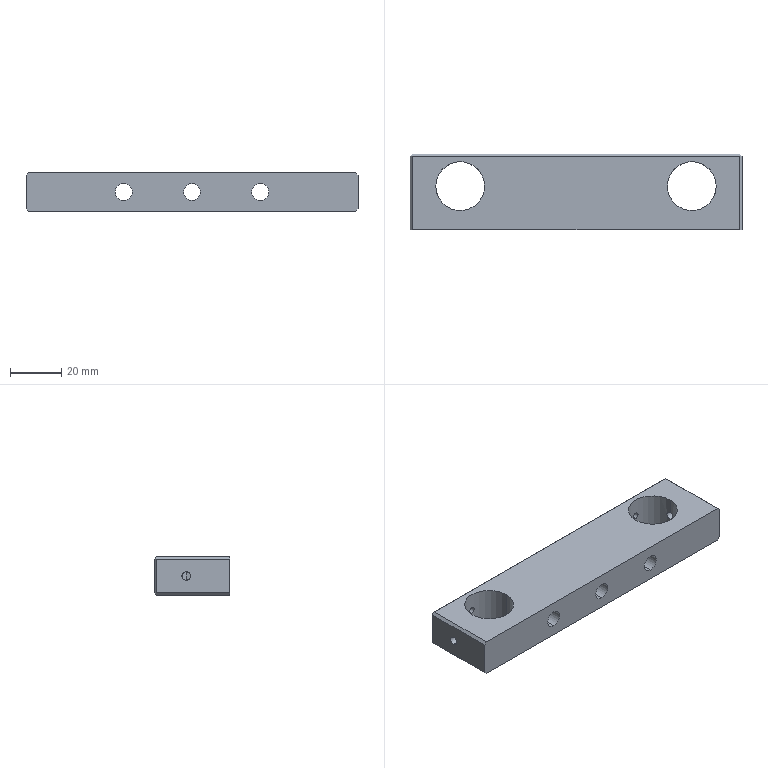Part | STEP file | PN_0008 Default | 1 solid | 41 faces | box 129 x 29.5 x 15 mm | volume 43870 mm3 | cylinder 24 | plane 17 | commonest cylinder face diameters 6.6 x6 11 x6 2.5 x4 3.3 x4 19 x4
STEP:
#1=CARTESIAN_POINT('',(-45.,26.5,6.25));
#2=VERTEX_POINT('',#1);
#3=CARTESIAN_POINT('',(-45.,26.5,8.75));
#4=VERTEX_POINT('',#3);
#5=CARTESIAN_POINT('',(-45.,26.5,6.25));
#6=CARTESIAN_POINT('',(-45.163,26.5,6.25));
#7=CARTESIAN_POINT('',(-45.328,26.496,6.283));
#8=CARTESIAN_POINT('',(-45.629,26.48,6.407));
#9=CARTESIAN_POINT('',(-45.768,26.47,6.5));
#10=CARTESIAN_POINT('',(-45.941,26.453,6.673));
#11=CARTESIAN_POINT('',(-45.994,26.448,6.737));
#12=CARTESIAN_POINT('',(-46.084,26.438,6.873));
#13=CARTESIAN_POINT('',(-46.123,26.433,6.945));
#14=CARTESIAN_POINT('',(-46.217,26.422,7.172));
#15=CARTESIAN_POINT('',(-46.25,26.417,7.334));
#16=CARTESIAN_POINT('',(-46.25,26.417,7.664));
#17=CARTESIAN_POINT('',(-46.218,26.422,7.827));
#18=CARTESIAN_POINT('',(-46.092,26.437,8.129));
#19=CARTESIAN_POINT('',(-46.,26.448,8.268));
#20=CARTESIAN_POINT('',(-45.769,26.469,8.498));
#21=CARTESIAN_POINT('',(-45.63,26.48,8.592));
#22=CARTESIAN_POINT('',(-45.33,26.495,8.717));
#23=CARTESIAN_POINT('',(-45.165,26.5,8.75));
#24=CARTESIAN_POINT('',(-45.,26.5,8.75));
#25=B_SPLINE_CURVE_WITH_KNOTS('',3,(#5,#6,#7,#8,#9,#10,#11,#12,#13,#14,#15,#16,#17,#18,#19,#20,#21,#22,#23,#24),.UNSPECIFIED.,.F.,.F.,(4,2,2,2,2,2,2,2,2,4),(0.003912,0.004401,0.00489,0.005135,0.005379,0.005868,0.006357,0.006846,0.007335,0.007824),.UNSPECIFIED.);
#26=EDGE_CURVE('',#2,#4,#25,.T.);
#27=ORIENTED_EDGE('',*,*,#26,.F.);
#28=CARTESIAN_POINT('',(-45.,29.5,6.25));
#29=VERTEX_POINT('',#28);
#30=CARTESIAN_POINT('',(-45.,29.5,6.25));
#31=DIRECTION('',(0.,1.,0.));
#32=VECTOR('',#31,1000.);
#33=LINE('',#30,#32);
#34=EDGE_CURVE('',#2,#29,#33,.T.);
#35=ORIENTED_EDGE('',*,*,#34,.T.);
#36=CARTESIAN_POINT('',(-45.,29.5,8.75));
#37=VERTEX_POINT('',#36);
#38=CARTESIAN_POINT('',(-45.,29.5,7.5));
#39=DIRECTION('',(0.,1.,0.));
#40=DIRECTION('',(0.,0.,1.));
#41=AXIS2_PLACEMENT_3D('',#38,#39,#40);
#42=CIRCLE('',#41,1.25);
#43=EDGE_CURVE('',#29,#37,#42,.T.);
#44=ORIENTED_EDGE('',*,*,#43,.T.);
#45=CARTESIAN_POINT('',(-45.,29.5,8.75));
#46=DIRECTION('',(0.,1.,0.));
#47=VECTOR('',#46,1000.);
#48=LINE('',#45,#47);
#49=EDGE_CURVE('',#4,#37,#48,.T.);
#50=ORIENTED_EDGE('',*,*,#49,.F.);
#51=EDGE_LOOP('',(#27,#35,#44,#50));
#52=FACE_OUTER_BOUND('',#51,.T.);
#53=CARTESIAN_POINT('',(-45.,29.5,7.5));
#54=DIRECTION('',(0.,1.,0.));
#55=DIRECTION('',(0.,0.,1.));
#56=AXIS2_PLACEMENT_3D('',#53,#54,#55);
#57=CYLINDRICAL_SURFACE('',#56,1.25);
#58=ADVANCED_FACE('',(#52),#57,.F.);
#59=CARTESIAN_POINT('',(0.,22.5,2.));
#60=VERTEX_POINT('',#59);
#61=CARTESIAN_POINT('',(0.,22.5,13.));
#62=VERTEX_POINT('',#61);
#63=CARTESIAN_POINT('',(0.,22.5,7.5));
#64=DIRECTION('',(0.,1.,0.));
#65=DIRECTION('',(0.,0.,1.));
#66=AXIS2_PLACEMENT_3D('',#63,#64,#65);
#67=CIRCLE('',#66,5.5);
#68=EDGE_CURVE('',#60,#62,#67,.T.);
#69=ORIENTED_EDGE('',*,*,#68,.F.);
#70=CARTESIAN_POINT('',(0.,29.5,2.));
#71=VERTEX_POINT('',#70);
#72=CARTESIAN_POINT('',(0.,29.5,2.));
#73=DIRECTION('',(0.,1.,0.));
#74=VECTOR('',#73,1000.);
#75=LINE('',#72,#74);
#76=EDGE_CURVE('',#60,#71,#75,.T.);
#77=ORIENTED_EDGE('',*,*,#76,.T.);
#78=CARTESIAN_POINT('',(0.,29.5,13.));
#79=VERTEX_POINT('',#78);
#80=CARTESIAN_POINT('',(0.,29.5,7.5));
#81=DIRECTION('',(0.,1.,0.));
#82=DIRECTION('',(0.,0.,1.));
#83=AXIS2_PLACEMENT_3D('',#80,#81,#82);
#84=CIRCLE('',#83,5.5);
#85=EDGE_CURVE('',#71,#79,#84,.T.);
#86=ORIENTED_EDGE('',*,*,#85,.T.);
#87=CARTESIAN_POINT('',(0.,29.5,13.));
#88=DIRECTION('',(0.,1.,0.));
#89=VECTOR('',#88,1000.);
#90=LINE('',#87,#89);
#91=EDGE_CURVE('',#62,#79,#90,.T.);
#92=ORIENTED_EDGE('',*,*,#91,.F.);
#93=EDGE_LOOP('',(#69,#77,#86,#92));
#94=FACE_OUTER_BOUND('',#93,.T.);
#95=CARTESIAN_POINT('',(0.,29.5,7.5));
#96=DIRECTION('',(0.,1.,0.));
#97=DIRECTION('',(0.,0.,1.));
#98=AXIS2_PLACEMENT_3D('',#95,#96,#97);
#99=CYLINDRICAL_SURFACE('',#98,5.5);
#100=ADVANCED_FACE('',(#94),#99,.F.);
#101=CARTESIAN_POINT('',(0.,0.,4.2));
#102=VERTEX_POINT('',#101);
#103=CARTESIAN_POINT('',(0.,0.,10.8));
#104=VERTEX_POINT('',#103);
#105=CARTESIAN_POINT('',(0.,0.,7.5));
#106=DIRECTION('',(0.,1.,0.));
#107=DIRECTION('',(0.,0.,1.));
#108=AXIS2_PLACEMENT_3D('',#105,#106,#107);
#109=CIRCLE('',#108,3.3);
#110=EDGE_CURVE('',#102,#104,#109,.T.);
#111=ORIENTED_EDGE('',*,*,#110,.F.);
#112=CARTESIAN_POINT('',(0.,22.5,4.2));
#113=VERTEX_POINT('',#112);
#114=CARTESIAN_POINT('',(0.,29.5,4.2));
#115=DIRECTION('',(0.,1.,0.));
#116=VECTOR('',#115,1000.);
#117=LINE('',#114,#116);
#118=EDGE_CURVE('',#102,#113,#117,.T.);
#119=ORIENTED_EDGE('',*,*,#118,.T.);
#120=CARTESIAN_POINT('',(0.,22.5,10.8));
#121=VERTEX_POINT('',#120);
#122=CARTESIAN_POINT('',(0.,22.5,7.5));
#123=DIRECTION('',(0.,1.,0.));
#124=DIRECTION('',(0.,0.,1.));
#125=AXIS2_PLACEMENT_3D('',#122,#123,#124);
#126=CIRCLE('',#125,3.3);
#127=EDGE_CURVE('',#113,#121,#126,.T.);
#128=ORIENTED_EDGE('',*,*,#127,.T.);
#129=CARTESIAN_POINT('',(0.,29.5,10.8));
#130=DIRECTION('',(0.,1.,0.));
#131=VECTOR('',#130,1000.);
#132=LINE('',#129,#131);
#133=EDGE_CURVE('',#104,#121,#132,.T.);
#134=ORIENTED_EDGE('',*,*,#133,.F.);
#135=EDGE_LOOP('',(#111,#119,#128,#134));
#136=FACE_OUTER_BOUND('',#135,.T.);
#137=CARTESIAN_POINT('',(0.,29.5,7.5));
#138=DIRECTION('',(0.,1.,0.));
#139=DIRECTION('',(0.,0.,1.));
#140=AXIS2_PLACEMENT_3D('',#137,#138,#139);
#141=CYLINDRICAL_SURFACE('',#140,3.3);
#142=ADVANCED_FACE('',(#136),#141,.F.);
#143=CARTESIAN_POINT('',(-26.5,22.5,2.));
#144=VERTEX_POINT('',#143);
#145=CARTESIAN_POINT('',(-26.5,22.5,13.));
#146=VERTEX_POINT('',#145);
#147=CARTESIAN_POINT('',(-26.5,22.5,7.5));
#148=DIRECTION('',(0.,1.,0.));
#149=DIRECTION('',(0.,0.,1.));
#150=AXIS2_PLACEMENT_3D('',#147,#148,#149);
#151=CIRCLE('',#150,5.5);
#152=EDGE_CURVE('',#144,#146,#151,.T.);
#153=ORIENTED_EDGE('',*,*,#152,.F.);
#154=CARTESIAN_POINT('',(-26.5,29.5,2.));
#155=VERTEX_POINT('',#154);
#156=CARTESIAN_POINT('',(-26.5,29.5,2.));
#157=DIRECTION('',(0.,1.,0.));
#158=VECTOR('',#157,1000.);
#159=LINE('',#156,#158);
#160=EDGE_CURVE('',#144,#155,#159,.T.);
#161=ORIENTED_EDGE('',*,*,#160,.T.);
#162=CARTESIAN_POINT('',(-26.5,29.5,13.));
#163=VERTEX_POINT('',#162);
#164=CARTESIAN_POINT('',(-26.5,29.5,7.5));
#165=DIRECTION('',(0.,1.,0.));
#166=DIRECTION('',(0.,0.,1.));
#167=AXIS2_PLACEMENT_3D('',#164,#165,#166);
#168=CIRCLE('',#167,5.5);
#169=EDGE_CURVE('',#155,#163,#168,.T.);
#170=ORIENTED_EDGE('',*,*,#169,.T.);
#171=CARTESIAN_POINT('',(-26.5,29.5,13.));
#172=DIRECTION('',(0.,1.,0.));
#173=VECTOR('',#172,1000.);
#174=LINE('',#171,#173);
#175=EDGE_CURVE('',#146,#163,#174,.T.);
#176=ORIENTED_EDGE('',*,*,#175,.F.);
#177=EDGE_LOOP('',(#153,#161,#170,#176));
#178=FACE_OUTER_BOUND('',#177,.T.);
#179=CARTESIAN_POINT('',(-26.5,29.5,7.5));
#180=DIRECTION('',(0.,1.,0.));
#181=DIRECTION('',(0.,0.,1.));
#182=AXIS2_PLACEMENT_3D('',#179,#180,#181);
#183=CYLINDRICAL_SURFACE('',#182,5.5);
#184=ADVANCED_FACE('',(#178),#183,.F.);
#185=CARTESIAN_POINT('',(-26.5,0.,4.2));
#186=VERTEX_POINT('',#185);
#187=CARTESIAN_POINT('',(-26.5,0.,10.8));
#188=VERTEX_POINT('',#187);
#189=CARTESIAN_POINT('',(-26.5,0.,7.5));
#190=DIRECTION('',(0.,1.,0.));
#191=DIRECTION('',(0.,0.,1.));
#192=AXIS2_PLACEMENT_3D('',#189,#190,#191);
#193=CIRCLE('',#192,3.3);
#194=EDGE_CURVE('',#186,#188,#193,.T.);
#195=ORIENTED_EDGE('',*,*,#194,.F.);
#196=CARTESIAN_POINT('',(-26.5,22.5,4.2));
#197=VERTEX_POINT('',#196);
#198=CARTESIAN_POINT('',(-26.5,29.5,4.2));
#199=DIRECTION('',(0.,1.,0.));
#200=VECTOR('',#199,1000.);
#201=LINE('',#198,#200);
#202=EDGE_CURVE('',#186,#197,#201,.T.);
#203=ORIENTED_EDGE('',*,*,#202,.T.);
#204=CARTESIAN_POINT('',(-26.5,22.5,10.8));
#205=VERTEX_POINT('',#204);
#206=CARTESIAN_POINT('',(-26.5,22.5,7.5));
#207=DIRECTION('',(0.,1.,0.));
#208=DIRECTION('',(0.,0.,1.));
#209=AXIS2_PLACEMENT_3D('',#206,#207,#208);
#210=CIRCLE('',#209,3.3);
#211=EDGE_CURVE('',#197,#205,#210,.T.);
#212=ORIENTED_EDGE('',*,*,#211,.T.);
#213=CARTESIAN_POINT('',(-26.5,29.5,10.8));
#214=DIRECTION('',(0.,1.,0.));
#215=VECTOR('',#214,1000.);
#216=LINE('',#213,#215);
#217=EDGE_CURVE('',#188,#205,#216,.T.);
#218=ORIENTED_EDGE('',*,*,#217,.F.);
#219=EDGE_LOOP('',(#195,#203,#212,#218));
#220=FACE_OUTER_BOUND('',#219,.T.);
#221=CARTESIAN_POINT('',(-26.5,29.5,7.5));
#222=DIRECTION('',(0.,1.,0.));
#223=DIRECTION('',(0.,0.,1.));
#224=AXIS2_PLACEMENT_3D('',#221,#222,#223);
#225=CYLINDRICAL_SURFACE('',#224,3.3);
#226=ADVANCED_FACE('',(#220),#225,.F.);
#227=CARTESIAN_POINT('',(26.5,22.5,2.));
#228=VERTEX_POINT('',#227);
#229=CARTESIAN_POINT('',(26.5,22.5,13.));
#230=VERTEX_POINT('',#229);
#231=CARTESIAN_POINT('',(26.5,22.5,7.5));
#232=DIRECTION('',(0.,1.,0.));
#233=DIRECTION('',(0.,0.,1.));
#234=AXIS2_PLACEMENT_3D('',#231,#232,#233);
#235=CIRCLE('',#234,5.5);
#236=EDGE_CURVE('',#228,#230,#235,.T.);
#237=ORIENTED_EDGE('',*,*,#236,.F.);
#238=CARTESIAN_POINT('',(26.5,29.5,2.));
#239=VERTEX_POINT('',#238);
#240=CARTESIAN_POINT('',(26.5,29.5,2.));
#241=DIRECTION('',(0.,1.,0.));
#242=VECTOR('',#241,1000.);
#243=LINE('',#240,#242);
#244=EDGE_CURVE('',#228,#239,#243,.T.);
#245=ORIENTED_EDGE('',*,*,#244,.T.);
#246=CARTESIAN_POINT('',(26.5,29.5,13.));
#247=VERTEX_POINT('',#246);
#248=CARTESIAN_POINT('',(26.5,29.5,7.5));
#249=DIRECTION('',(0.,1.,0.));
#250=DIRECTION('',(0.,0.,1.));
#251=AXIS2_PLACEMENT_3D('',#248,#249,#250);
#252=CIRCLE('',#251,5.5);
#253=EDGE_CURVE('',#239,#247,#252,.T.);
#254=ORIENTED_EDGE('',*,*,#253,.T.);
#255=CARTESIAN_POINT('',(26.5,29.5,13.));
#256=DIRECTION('',(0.,1.,0.));
#257=VECTOR('',#256,1000.);
#258=LINE('',#255,#257);
#259=EDGE_CURVE('',#230,#247,#258,.T.);
#260=ORIENTED_EDGE('',*,*,#259,.F.);
#261=EDGE_LOOP('',(#237,#245,#254,#260));
#262=FACE_OUTER_BOUND('',#261,.T.);
#263=CARTESIAN_POINT('',(26.5,29.5,7.5));
#264=DIRECTION('',(0.,1.,0.));
#265=DIRECTION('',(0.,0.,1.));
#266=AXIS2_PLACEMENT_3D('',#263,#264,#265);
#267=CYLINDRICAL_SURFACE('',#266,5.5);
#268=ADVANCED_FACE('',(#262),#267,.F.);
#269=CARTESIAN_POINT('',(26.5,0.,4.2));
#270=VERTEX_POINT('',#269);
#271=CARTESIAN_POINT('',(26.5,0.,10.8));
#272=VERTEX_POINT('',#271);
#273=CARTESIAN_POINT('',(26.5,0.,7.5));
#274=DIRECTION('',(0.,1.,0.));
#275=DIRECTION('',(0.,0.,1.));
#276=AXIS2_PLACEMENT_3D('',#273,#274,#275);
#277=CIRCLE('',#276,3.3);
#278=EDGE_CURVE('',#270,#272,#277,.T.);
#279=ORIENTED_EDGE('',*,*,#278,.F.);
#280=CARTESIAN_POINT('',(26.5,22.5,4.2));
#281=VERTEX_POINT('',#280);
#282=CARTESIAN_POINT('',(26.5,29.5,4.2));
#283=DIRECTION('',(0.,1.,0.));
#284=VECTOR('',#283,1000.);
#285=LINE('',#282,#284);
#286=EDGE_CURVE('',#270,#281,#285,.T.);
#287=ORIENTED_EDGE('',*,*,#286,.T.);
#288=CARTESIAN_POINT('',(26.5,22.5,10.8));
#289=VERTEX_POINT('',#288);
#290=CARTESIAN_POINT('',(26.5,22.5,7.5));
#291=DIRECTION('',(0.,1.,0.));
#292=DIRECTION('',(0.,0.,1.));
#293=AXIS2_PLACEMENT_3D('',#290,#291,#292);
#294=CIRCLE('',#293,3.3);
#295=EDGE_CURVE('',#281,#289,#294,.T.);
#296=ORIENTED_EDGE('',*,*,#295,.T.);
#297=CARTESIAN_POINT('',(26.5,29.5,10.8));
#298=DIRECTION('',(0.,1.,0.));
#299=VECTOR('',#298,1000.);
#300=LINE('',#297,#299);
#301=EDGE_CURVE('',#272,#289,#300,.T.);
#302=ORIENTED_EDGE('',*,*,#301,.F.);
#303=EDGE_LOOP('',(#279,#287,#296,#302));
#304=FACE_OUTER_BOUND('',#303,.T.);
#305=CARTESIAN_POINT('',(26.5,29.5,7.5));
#306=DIRECTION('',(0.,1.,0.));
#307=DIRECTION('',(0.,0.,1.));
#308=AXIS2_PLACEMENT_3D('',#305,#306,#307);
#309=CYLINDRICAL_SURFACE('',#308,3.3);
#310=ADVANCED_FACE('',(#304),#309,.F.);
#311=CARTESIAN_POINT('',(45.,26.5,6.25));
#312=VERTEX_POINT('',#311);
#313=CARTESIAN_POINT('',(45.,26.5,8.75));
#314=VERTEX_POINT('',#313);
#315=CARTESIAN_POINT('',(45.,26.5,6.25));
#316=CARTESIAN_POINT('',(44.837,26.5,6.25));
#317=CARTESIAN_POINT('',(44.672,26.496,6.283));
#318=CARTESIAN_POINT('',(44.371,26.48,6.407));
#319=CARTESIAN_POINT('',(44.232,26.47,6.5));
#320=CARTESIAN_POINT('',(44.059,26.453,6.673));
#321=CARTESIAN_POINT('',(44.006,26.448,6.737));
#322=CARTESIAN_POINT('',(43.916,26.438,6.873));
#323=CARTESIAN_POINT('',(43.877,26.433,6.945));
#324=CARTESIAN_POINT('',(43.783,26.422,7.172));
#325=CARTESIAN_POINT('',(43.75,26.417,7.334));
#326=CARTESIAN_POINT('',(43.75,26.417,7.664));
#327=CARTESIAN_POINT('',(43.782,26.422,7.827));
#328=CARTESIAN_POINT('',(43.908,26.437,8.129));
#329=CARTESIAN_POINT('',(44.,26.448,8.268));
#330=CARTESIAN_POINT('',(44.231,26.469,8.498));
#331=CARTESIAN_POINT('',(44.37,26.48,8.592));
#332=CARTESIAN_POINT('',(44.67,26.495,8.717));
#333=CARTESIAN_POINT('',(44.835,26.5,8.75));
#334=CARTESIAN_POINT('',(45.,26.5,8.75));
#335=B_SPLINE_CURVE_WITH_KNOTS('',3,(#315,#316,#317,#318,#319,#320,#321,#322,#323,#324,#325,#326,#327,#328,#329,#330,#331,#332,#333,#334),.UNSPECIFIED.,.F.,.F.,(4,2,2,2,2,2,2,2,2,4),(0.003912,0.004401,0.00489,0.005135,0.005379,0.005868,0.006357,0.006846,0.007335,0.007824),.UNSPECIFIED.);
#336=EDGE_CURVE('',#312,#314,#335,.T.);
#337=ORIENTED_EDGE('',*,*,#336,.F.);
#338=CARTESIAN_POINT('',(45.,29.5,6.25));
#339=VERTEX_POINT('',#338);
#340=CARTESIAN_POINT('',(45.,29.5,6.25));
#341=DIRECTION('',(0.,1.,0.));
#342=VECTOR('',#341,1000.);
#343=LINE('',#340,#342);
#344=EDGE_CURVE('',#312,#339,#343,.T.);
#345=ORIENTED_EDGE('',*,*,#344,.T.);
#346=CARTESIAN_POINT('',(45.,29.5,8.75));
#347=VERTEX_POINT('',#346);
#348=CARTESIAN_POINT('',(45.,29.5,7.5));
#349=DIRECTION('',(0.,1.,0.));
#350=DIRECTION('',(0.,0.,1.));
#351=AXIS2_PLACEMENT_3D('',#348,#349,#350);
#352=CIRCLE('',#351,1.25);
#353=EDGE_CURVE('',#339,#347,#352,.T.);
#354=ORIENTED_EDGE('',*,*,#353,.T.);
#355=CARTESIAN_POINT('',(45.,29.5,8.75));
#356=DIRECTION('',(0.,1.,0.));
#357=VECTOR('',#356,1000.);
#358=LINE('',#355,#357);
#359=EDGE_CURVE('',#314,#347,#358,.T.);
#360=ORIENTED_EDGE('',*,*,#359,.F.);
#361=EDGE_LOOP('',(#337,#345,#354,#360));
#362=FACE_OUTER_BOUND('',#361,.T.);
#363=CARTESIAN_POINT('',(45.,29.5,7.5));
#364=DIRECTION('',(0.,1.,0.));
#365=DIRECTION('',(0.,0.,1.));
#366=AXIS2_PLACEMENT_3D('',#363,#364,#365);
#367=CYLINDRICAL_SURFACE('',#366,1.25);
#368=ADVANCED_FACE('',(#362),#367,.F.);
#369=CARTESIAN_POINT('',(-54.5,17.,5.85));
#370=VERTEX_POINT('',#369);
#371=CARTESIAN_POINT('',(-54.5,17.,9.15));
#372=VERTEX_POINT('',#371);
#373=CARTESIAN_POINT('',(-54.5,17.,5.85));
#374=CARTESIAN_POINT('',(-54.5,16.784,5.85));
#375=CARTESIAN_POINT('',(-54.492,16.567,5.893));
#376=CARTESIAN_POINT('',(-54.466,16.17,6.058));
#377=CARTESIAN_POINT('',(-54.447,15.986,6.181));
#378=CARTESIAN_POINT('',(-54.419,15.758,6.409));
#379=CARTESIAN_POINT('',(-54.409,15.688,6.493));
#380=CARTESIAN_POINT('',(-54.392,15.569,6.672));
#381=CARTESIAN_POINT('',(-54.384,15.518,6.767));
#382=CARTESIAN_POINT('',(-54.364,15.393,7.067));
#383=CARTESIAN_POINT('',(-54.356,15.35,7.281));
#384=CARTESIAN_POINT('',(-54.356,15.35,7.608));
#385=CARTESIAN_POINT('',(-54.357,15.361,7.715));
#386=CARTESIAN_POINT('',(-54.365,15.402,7.927));
#387=CARTESIAN_POINT('',(-54.37,15.434,8.032));
#388=CARTESIAN_POINT('',(-54.384,15.517,8.231));
#389=CARTESIAN_POINT('',(-54.392,15.568,8.326));
#390=CARTESIAN_POINT('',(-54.409,15.687,8.505));
#391=CARTESIAN_POINT('',(-54.419,15.757,8.59));
#392=CARTESIAN_POINT('',(-54.447,15.984,8.818));
#393=CARTESIAN_POINT('',(-54.466,16.168,8.941));
#394=CARTESIAN_POINT('',(-54.492,16.565,9.106));
#395=CARTESIAN_POINT('',(-54.5,16.782,9.15));
#396=CARTESIAN_POINT('',(-54.5,17.,9.15));
#397=B_SPLINE_CURVE_WITH_KNOTS('',3,(#373,#374,#375,#376,#377,#378,#379,#380,#381,#382,#383,#384,#385,#386,#387,#388,#389,#390,#391,#392,#393,#394,#395,#396),.UNSPECIFIED.,.F.,.F.,(4,2,2,2,2,2,2,2,2,2,2,4),(0.005168,0.005814,0.00646,0.006783,0.007106,0.007752,0.008075,0.008398,0.008721,0.009044,0.00969,0.01034),.UNSPECIFIED.);
#398=EDGE_CURVE('',#370,#372,#397,.T.);
#399=ORIENTED_EDGE('',*,*,#398,.F.);
#400=CARTESIAN_POINT('',(-64.5,17.,5.85));
#401=VERTEX_POINT('',#400);
#402=CARTESIAN_POINT('',(-64.5,17.,5.85));
#403=DIRECTION('',(-1.,0.,0.));
#404=VECTOR('',#403,1000.);
#405=LINE('',#402,#404);
#406=EDGE_CURVE('',#370,#401,#405,.T.);
#407=ORIENTED_EDGE('',*,*,#406,.T.);
#408=CARTESIAN_POINT('',(-64.5,17.,9.15));
#409=VERTEX_POINT('',#408);
#410=CARTESIAN_POINT('',(-64.5,17.,7.5));
#411=DIRECTION('',(-1.,0.,0.));
#412=DIRECTION('',(0.,0.,1.));
#413=AXIS2_PLACEMENT_3D('',#410,#411,#412);
#414=CIRCLE('',#413,1.65);
#415=EDGE_CURVE('',#401,#409,#414,.T.);
#416=ORIENTED_EDGE('',*,*,#415,.T.);
#417=CARTESIAN_POINT('',(-64.5,17.,9.15));
#418=DIRECTION('',(-1.,0.,0.));
#419=VECTOR('',#418,1000.);
#420=LINE('',#417,#419);
#421=EDGE_CURVE('',#372,#409,#420,.T.);
#422=ORIENTED_EDGE('',*,*,#421,.F.);
#423=EDGE_LOOP('',(#399,#407,#416,#422));
#424=FACE_OUTER_BOUND('',#423,.T.);
#425=CARTESIAN_POINT('',(-64.5,17.,7.5));
#426=DIRECTION('',(-1.,0.,0.));
#427=DIRECTION('',(0.,0.,1.));
#428=AXIS2_PLACEMENT_3D('',#425,#426,#427);
#429=CYLINDRICAL_SURFACE('',#428,1.65);
#430=ADVANCED_FACE('',(#424),#429,.F.);
#431=CARTESIAN_POINT('',(54.5,17.,9.15));
#432=VERTEX_POINT('',#431);
#433=CARTESIAN_POINT('',(54.5,17.,5.85));
#434=VERTEX_POINT('',#433);
#435=CARTESIAN_POINT('',(54.5,17.,9.15));
#436=CARTESIAN_POINT('',(54.5,16.784,9.15));
#437=CARTESIAN_POINT('',(54.492,16.567,9.107));
#438=CARTESIAN_POINT('',(54.466,16.17,8.942));
#439=CARTESIAN_POINT('',(54.447,15.986,8.819));
#440=CARTESIAN_POINT('',(54.419,15.758,8.591));
#441=CARTESIAN_POINT('',(54.409,15.688,8.507));
#442=CARTESIAN_POINT('',(54.392,15.569,8.328));
#443=CARTESIAN_POINT('',(54.384,15.518,8.233));
#444=CARTESIAN_POINT('',(54.364,15.393,7.933));
#445=CARTESIAN_POINT('',(54.356,15.35,7.719));
#446=CARTESIAN_POINT('',(54.356,15.35,7.392));
#447=CARTESIAN_POINT('',(54.357,15.361,7.285));
#448=CARTESIAN_POINT('',(54.365,15.402,7.073));
#449=CARTESIAN_POINT('',(54.37,15.434,6.968));
#450=CARTESIAN_POINT('',(54.384,15.517,6.769));
#451=CARTESIAN_POINT('',(54.392,15.568,6.674));
#452=CARTESIAN_POINT('',(54.409,15.687,6.495));
#453=CARTESIAN_POINT('',(54.419,15.757,6.41));
#454=CARTESIAN_POINT('',(54.447,15.984,6.182));
#455=CARTESIAN_POINT('',(54.466,16.168,6.059));
#456=CARTESIAN_POINT('',(54.492,16.565,5.894));
#457=CARTESIAN_POINT('',(54.5,16.782,5.85));
#458=CARTESIAN_POINT('',(54.5,17.,5.85));
#459=B_SPLINE_CURVE_WITH_KNOTS('',3,(#435,#436,#437,#438,#439,#440,#441,#442,#443,#444,#445,#446,#447,#448,#449,#450,#451,#452,#453,#454,#455,#456,#457,#458),.UNSPECIFIED.,.F.,.F.,(4,2,2,2,2,2,2,2,2,2,2,4),(0.005168,0.005814,0.00646,0.006783,0.007106,0.007752,0.008075,0.008398,0.008721,0.009044,0.00969,0.01034),.UNSPECIFIED.);
#460=EDGE_CURVE('',#432,#434,#459,.T.);
#461=ORIENTED_EDGE('',*,*,#460,.F.);
#462=CARTESIAN_POINT('',(64.5,17.,9.15));
#463=VERTEX_POINT('',#462);
#464=CARTESIAN_POINT('',(64.5,17.,9.15));
#465=DIRECTION('',(1.,0.,0.));
#466=VECTOR('',#465,1000.);
#467=LINE('',#464,#466);
#468=EDGE_CURVE('',#432,#463,#467,.T.);
#469=ORIENTED_EDGE('',*,*,#468,.T.);
#470=CARTESIAN_POINT('',(64.5,17.,5.85));
#471=VERTEX_POINT('',#470);
#472=CARTESIAN_POINT('',(64.5,17.,7.5));
#473=DIRECTION('',(1.,0.,0.));
#474=DIRECTION('',(0.,0.,-1.));
#475=AXIS2_PLACEMENT_3D('',#472,#473,#474);
#476=CIRCLE('',#475,1.65);
#477=EDGE_CURVE('',#463,#471,#476,.T.);
#478=ORIENTED_EDGE('',*,*,#477,.T.);
#479=CARTESIAN_POINT('',(64.5,17.,5.85));
#480=DIRECTION('',(1.,0.,0.));
#481=VECTOR('',#480,1000.);
#482=LINE('',#479,#481);
#483=EDGE_CURVE('',#434,#471,#482,.T.);
#484=ORIENTED_EDGE('',*,*,#483,.F.);
#485=EDGE_LOOP('',(#461,#469,#478,#484));
#486=FACE_OUTER_BOUND('',#485,.T.);
#487=CARTESIAN_POINT('',(64.5,17.,7.5));
#488=DIRECTION('',(1.,0.,0.));
#489=DIRECTION('',(0.,0.,-1.));
#490=AXIS2_PLACEMENT_3D('',#487,#488,#489);
#491=CYLINDRICAL_SURFACE('',#490,1.65);
#492=ADVANCED_FACE('',(#486),#491,.F.);
#493=CARTESIAN_POINT('',(54.5,17.,15.));
#494=VERTEX_POINT('',#493);
#495=CARTESIAN_POINT('',(35.5,17.,15.));
#496=VERTEX_POINT('',#495);
#497=CARTESIAN_POINT('',(45.,17.,15.));
#498=DIRECTION('',(0.,0.,-1.));
#499=DIRECTION('',(-1.,0.,0.));
#500=AXIS2_PLACEMENT_3D('',#497,#498,#499);
#501=CIRCLE('',#500,9.5);
#502=EDGE_CURVE('',#494,#496,#501,.T.);
#503=ORIENTED_EDGE('',*,*,#502,.F.);
#504=CARTESIAN_POINT('',(54.5,17.,15.));
#505=DIRECTION('',(0.,0.,-1.));
#506=VECTOR('',#505,1000.);
#507=LINE('',#504,#506);
#508=EDGE_CURVE('',#494,#432,#507,.T.);
#509=ORIENTED_EDGE('',*,*,#508,.T.);
#510=ORIENTED_EDGE('',*,*,#460,.T.);
#511=CARTESIAN_POINT('',(54.5,17.,0.));
#512=VERTEX_POINT('',#511);
#513=CARTESIAN_POINT('',(54.5,17.,15.));
#514=DIRECTION('',(0.,0.,-1.));
#515=VECTOR('',#514,1000.);
#516=LINE('',#513,#515);
#517=EDGE_CURVE('',#434,#512,#516,.T.);
#518=ORIENTED_EDGE('',*,*,#517,.T.);
#519=CARTESIAN_POINT('',(35.5,17.,0.));
#520=VERTEX_POINT('',#519);
#521=CARTESIAN_POINT('',(45.,17.,0.));
#522=DIRECTION('',(0.,0.,-1.));
#523=DIRECTION('',(-1.,0.,0.));
#524=AXIS2_PLACEMENT_3D('',#521,#522,#523);
#525=CIRCLE('',#524,9.5);
#526=EDGE_CURVE('',#512,#520,#525,.T.);
#527=ORIENTED_EDGE('',*,*,#526,.T.);
#528=CARTESIAN_POINT('',(35.5,17.,15.));
#529=DIRECTION('',(0.,0.,-1.));
#530=VECTOR('',#529,1000.);
#531=LINE('',#528,#530);
#532=EDGE_CURVE('',#496,#520,#531,.T.);
#533=ORIENTED_EDGE('',*,*,#532,.F.);
#534=EDGE_LOOP('',(#503,#509,#510,#518,#527,#533));
#535=FACE_OUTER_BOUND('',#534,.T.);
#536=CARTESIAN_POINT('',(45.,17.,15.));
#537=DIRECTION('',(0.,0.,-1.));
#538=DIRECTION('',(-1.,0.,0.));
#539=AXIS2_PLACEMENT_3D('',#536,#537,#538);
#540=CYLINDRICAL_SURFACE('',#539,9.5);
#541=ADVANCED_FACE('',(#535),#540,.F.);
#542=CARTESIAN_POINT('',(-35.5,17.,15.));
#543=VERTEX_POINT('',#542);
#544=CARTESIAN_POINT('',(-54.5,17.,15.));
#545=VERTEX_POINT('',#544);
#546=CARTESIAN_POINT('',(-45.,17.,15.));
#547=DIRECTION('',(0.,0.,-1.));
#548=DIRECTION('',(-1.,0.,0.));
#549=AXIS2_PLACEMENT_3D('',#546,#547,#548);
#550=CIRCLE('',#549,9.5);
#551=EDGE_CURVE('',#543,#545,#550,.T.);
#552=ORIENTED_EDGE('',*,*,#551,.F.);
#553=CARTESIAN_POINT('',(-35.5,17.,0.));
#554=VERTEX_POINT('',#553);
#555=CARTESIAN_POINT('',(-35.5,17.,15.));
#556=DIRECTION('',(0.,0.,-1.));
#557=VECTOR('',#556,1000.);
#558=LINE('',#555,#557);
#559=EDGE_CURVE('',#543,#554,#558,.T.);
#560=ORIENTED_EDGE('',*,*,#559,.T.);
#561=CARTESIAN_POINT('',(-54.5,17.,0.));
#562=VERTEX_POINT('',#561);
#563=CARTESIAN_POINT('',(-45.,17.,0.));
#564=DIRECTION('',(0.,0.,-1.));
#565=DIRECTION('',(-1.,0.,0.));
#566=AXIS2_PLACEMENT_3D('',#563,#564,#565);
#567=CIRCLE('',#566,9.5);
#568=EDGE_CURVE('',#554,#562,#567,.T.);
#569=ORIENTED_EDGE('',*,*,#568,.T.);
#570=CARTESIAN_POINT('',(-54.5,17.,15.));
#571=DIRECTION('',(0.,0.,-1.));
#572=VECTOR('',#571,1000.);
#573=LINE('',#570,#572);
#574=EDGE_CURVE('',#370,#562,#573,.T.);
#575=ORIENTED_EDGE('',*,*,#574,.F.);
#576=ORIENTED_EDGE('',*,*,#398,.T.);
#577=CARTESIAN_POINT('',(-54.5,17.,15.));
#578=DIRECTION('',(0.,0.,-1.));
#579=VECTOR('',#578,1000.);
#580=LINE('',#577,#579);
#581=EDGE_CURVE('',#545,#372,#580,.T.);
#582=ORIENTED_EDGE('',*,*,#581,.F.);
#583=EDGE_LOOP('',(#552,#560,#569,#575,#576,#582));
#584=FACE_OUTER_BOUND('',#583,.T.);
#585=CARTESIAN_POINT('',(-45.,17.,15.));
#586=DIRECTION('',(0.,0.,-1.));
#587=DIRECTION('',(-1.,0.,0.));
#588=AXIS2_PLACEMENT_3D('',#585,#586,#587);
#589=CYLINDRICAL_SURFACE('',#588,9.5);
#590=ADVANCED_FACE('',(#584),#589,.F.);
#591=CARTESIAN_POINT('',(-64.5,17.,7.5));
#592=DIRECTION('',(-1.,0.,0.));
#593=DIRECTION('',(0.,0.,1.));
#594=AXIS2_PLACEMENT_3D('',#591,#592,#593);
#595=CIRCLE('',#594,1.65);
#596=EDGE_CURVE('',#409,#401,#595,.T.);
#597=ORIENTED_EDGE('',*,*,#596,.F.);
#598=ORIENTED_EDGE('',*,*,#415,.F.);
#599=EDGE_LOOP('',(#597,#598));
#600=FACE_BOUND('',#599,.T.);
#601=CARTESIAN_POINT('',(-64.5,28.5,14.));
#602=VERTEX_POINT('',#601);
#603=CARTESIAN_POINT('',(-64.5,28.5,1.));
#604=VERTEX_POINT('',#603);
#605=CARTESIAN_POINT('',(-64.5,28.5,15.));
#606=DIRECTION('',(0.,0.,-1.));
#607=VECTOR('',#606,1000.);
#608=LINE('',#605,#607);
#609=EDGE_CURVE('',#602,#604,#608,.T.);
#610=ORIENTED_EDGE('',*,*,#609,.T.);
#611=CARTESIAN_POINT('',(-64.5,0.,1.));
#612=VERTEX_POINT('',#611);
#613=CARTESIAN_POINT('',(-64.5,0.,1.));
#614=DIRECTION('',(0.,-1.,0.));
#615=VECTOR('',#614,1000.);
#616=LINE('',#613,#615);
#617=EDGE_CURVE('',#604,#612,#616,.T.);
#618=ORIENTED_EDGE('',*,*,#617,.T.);
#619=CARTESIAN_POINT('',(-64.5,0.,14.));
#620=VERTEX_POINT('',#619);
#621=CARTESIAN_POINT('',(-64.5,0.,15.));
#622=DIRECTION('',(0.,0.,-1.));
#623=VECTOR('',#622,1000.);
#624=LINE('',#621,#623);
#625=EDGE_CURVE('',#620,#612,#624,.T.);
#626=ORIENTED_EDGE('',*,*,#625,.F.);
#627=CARTESIAN_POINT('',(-64.5,0.,14.));
#628=DIRECTION('',(0.,1.,0.));
#629=VECTOR('',#628,1000.);
#630=LINE('',#627,#629);
#631=EDGE_CURVE('',#620,#602,#630,.T.);
#632=ORIENTED_EDGE('',*,*,#631,.T.);
#633=EDGE_LOOP('',(#610,#618,#626,#632));
#634=FACE_OUTER_BOUND('',#633,.T.);
#635=CARTESIAN_POINT('',(-64.5,0.,15.));
#636=DIRECTION('',(1.,0.,0.));
#637=DIRECTION('',(0.,0.,-1.));
#638=AXIS2_PLACEMENT_3D('',#635,#636,#637);
#639=PLANE('',#638);
#640=ADVANCED_FACE('',(#600,#634),#639,.F.);
#641=CARTESIAN_POINT('',(0.,0.,7.5));
#642=DIRECTION('',(0.,1.,0.));
#643=DIRECTION('',(0.,0.,1.));
#644=AXIS2_PLACEMENT_3D('',#641,#642,#643);
#645=CIRCLE('',#644,3.3);
#646=EDGE_CURVE('',#104,#102,#645,.T.);
#647=ORIENTED_EDGE('',*,*,#646,.T.);
#648=ORIENTED_EDGE('',*,*,#110,.T.);
#649=EDGE_LOOP('',(#647,#648));
#650=FACE_BOUND('',#649,.T.);
#651=CARTESIAN_POINT('',(-26.5,0.,7.5));
#652=DIRECTION('',(0.,1.,0.));
#653=DIRECTION('',(0.,0.,1.));
#654=AXIS2_PLACEMENT_3D('',#651,#652,#653);
#655=CIRCLE('',#654,3.3);
#656=EDGE_CURVE('',#188,#186,#655,.T.);
#657=ORIENTED_EDGE('',*,*,#656,.T.);
#658=ORIENTED_EDGE('',*,*,#194,.T.);
#659=EDGE_LOOP('',(#657,#658));
#660=FACE_BOUND('',#659,.T.);
#661=CARTESIAN_POINT('',(26.5,0.,7.5));
#662=DIRECTION('',(0.,1.,0.));
#663=DIRECTION('',(0.,0.,1.));
#664=AXIS2_PLACEMENT_3D('',#661,#662,#663);
#665=CIRCLE('',#664,3.3);
#666=EDGE_CURVE('',#272,#270,#665,.T.);
#667=ORIENTED_EDGE('',*,*,#666,.T.);
#668=ORIENTED_EDGE('',*,*,#278,.T.);
#669=EDGE_LOOP('',(#667,#668));
#670=FACE_BOUND('',#669,.T.);
#671=ORIENTED_EDGE('',*,*,#625,.T.);
#672=CARTESIAN_POINT('',(-63.5,0.,0.));
#673=VERTEX_POINT('',#672);
#674=CARTESIAN_POINT('',(-64.5,0.,1.));
#675=DIRECTION('',(0.7071,0.,-0.7071));
#676=VECTOR('',#675,1000.);
#677=LINE('',#674,#676);
#678=EDGE_CURVE('',#612,#673,#677,.T.);
#679=ORIENTED_EDGE('',*,*,#678,.T.);
#680=CARTESIAN_POINT('',(63.5,0.,0.));
#681=VERTEX_POINT('',#680);
#682=CARTESIAN_POINT('',(-64.5,0.,0.));
#683=DIRECTION('',(1.,0.,0.));
#684=VECTOR('',#683,1000.);
#685=LINE('',#682,#684);
#686=EDGE_CURVE('',#673,#681,#685,.T.);
#687=ORIENTED_EDGE('',*,*,#686,.T.);
#688=CARTESIAN_POINT('',(64.5,0.,1.));
#689=VERTEX_POINT('',#688);
#690=CARTESIAN_POINT('',(64.5,0.,1.));
#691=DIRECTION('',(0.7071,0.,0.7071));
#692=VECTOR('',#691,1000.);
#693=LINE('',#690,#692);
#694=EDGE_CURVE('',#681,#689,#693,.T.);
#695=ORIENTED_EDGE('',*,*,#694,.T.);
#696=CARTESIAN_POINT('',(64.5,0.,14.));
#697=VERTEX_POINT('',#696);
#698=CARTESIAN_POINT('',(64.5,0.,15.));
#699=DIRECTION('',(0.,0.,-1.));
#700=VECTOR('',#699,1000.);
#701=LINE('',#698,#700);
#702=EDGE_CURVE('',#697,#689,#701,.T.);
#703=ORIENTED_EDGE('',*,*,#702,.F.);
#704=CARTESIAN_POINT('',(63.5,0.,15.));
#705=VERTEX_POINT('',#704);
#706=CARTESIAN_POINT('',(63.5,0.,15.));
#707=DIRECTION('',(-0.7071,0.,0.7071));
#708=VECTOR('',#707,1000.);
#709=LINE('',#706,#708);
#710=EDGE_CURVE('',#697,#705,#709,.T.);
#711=ORIENTED_EDGE('',*,*,#710,.T.);
#712=CARTESIAN_POINT('',(-63.5,0.,15.));
#713=VERTEX_POINT('',#712);
#714=CARTESIAN_POINT('',(-64.5,0.,15.));
#715=DIRECTION('',(1.,0.,0.));
#716=VECTOR('',#715,1000.);
#717=LINE('',#714,#716);
#718=EDGE_CURVE('',#713,#705,#717,.T.);
#719=ORIENTED_EDGE('',*,*,#718,.F.);
#720=CARTESIAN_POINT('',(-63.5,0.,15.));
#721=DIRECTION('',(-0.7071,0.,-0.7071));
#722=VECTOR('',#721,1000.);
#723=LINE('',#720,#722);
#724=EDGE_CURVE('',#713,#620,#723,.T.);
#725=ORIENTED_EDGE('',*,*,#724,.T.);
#726=EDGE_LOOP('',(#671,#679,#687,#695,#703,#711,#719,#725));
#727=FACE_OUTER_BOUND('',#726,.T.);
#728=CARTESIAN_POINT('',(-64.5,0.,15.));
#729=DIRECTION('',(0.,1.,0.));
#730=DIRECTION('',(-1.,0.,0.));
#731=AXIS2_PLACEMENT_3D('',#728,#729,#730);
#732=PLANE('',#731);
#733=ADVANCED_FACE('',(#650,#660,#670,#727),#732,.F.);
#734=CARTESIAN_POINT('',(64.5,17.,7.5));
#735=DIRECTION('',(1.,0.,0.));
#736=DIRECTION('',(0.,0.,-1.));
#737=AXIS2_PLACEMENT_3D('',#734,#735,#736);
#738=CIRCLE('',#737,1.65);
#739=EDGE_CURVE('',#471,#463,#738,.T.);
#740=ORIENTED_EDGE('',*,*,#739,.F.);
#741=ORIENTED_EDGE('',*,*,#477,.F.);
#742=EDGE_LOOP('',(#740,#741));
#743=FACE_BOUND('',#742,.T.);
#744=ORIENTED_EDGE('',*,*,#702,.T.);
#745=CARTESIAN_POINT('',(64.5,28.5,1.));
#746=VERTEX_POINT('',#745);
#747=CARTESIAN_POINT('',(64.5,28.5,1.));
#748=DIRECTION('',(0.,1.,0.));
#749=VECTOR('',#748,1000.);
#750=LINE('',#747,#749);
#751=EDGE_CURVE('',#689,#746,#750,.T.);
#752=ORIENTED_EDGE('',*,*,#751,.T.);
#753=CARTESIAN_POINT('',(64.5,28.5,14.));
#754=VERTEX_POINT('',#753);
#755=CARTESIAN_POINT('',(64.5,28.5,15.));
#756=DIRECTION('',(0.,0.,1.));
#757=VECTOR('',#756,1000.);
#758=LINE('',#755,#757);
#759=EDGE_CURVE('',#746,#754,#758,.T.);
#760=ORIENTED_EDGE('',*,*,#759,.T.);
#761=CARTESIAN_POINT('',(64.5,0.,14.));
#762=DIRECTION('',(0.,-1.,0.));
#763=VECTOR('',#762,1000.);
#764=LINE('',#761,#763);
#765=EDGE_CURVE('',#754,#697,#764,.T.);
#766=ORIENTED_EDGE('',*,*,#765,.T.);
#767=EDGE_LOOP('',(#744,#752,#760,#766));
#768=FACE_OUTER_BOUND('',#767,.T.);
#769=CARTESIAN_POINT('',(64.5,0.,15.));
#770=DIRECTION('',(-1.,0.,0.));
#771=DIRECTION('',(0.,0.,1.));
#772=AXIS2_PLACEMENT_3D('',#769,#770,#771);
#773=PLANE('',#772);
#774=ADVANCED_FACE('',(#743,#768),#773,.F.);
#775=CARTESIAN_POINT('',(45.,17.,15.));
#776=DIRECTION('',(0.,0.,-1.));
#777=DIRECTION('',(-1.,0.,0.));
#778=AXIS2_PLACEMENT_3D('',#775,#776,#777);
#779=CIRCLE('',#778,9.5);
#780=EDGE_CURVE('',#496,#494,#779,.T.);
#781=ORIENTED_EDGE('',*,*,#780,.T.);
#782=ORIENTED_EDGE('',*,*,#502,.T.);
#783=EDGE_LOOP('',(#781,#782));
#784=FACE_BOUND('',#783,.T.);
#785=CARTESIAN_POINT('',(-45.,17.,15.));
#786=DIRECTION('',(0.,0.,-1.));
#787=DIRECTION('',(-1.,0.,0.));
#788=AXIS2_PLACEMENT_3D('',#785,#786,#787);
#789=CIRCLE('',#788,9.5);
#790=EDGE_CURVE('',#545,#543,#789,.T.);
#791=ORIENTED_EDGE('',*,*,#790,.T.);
#792=ORIENTED_EDGE('',*,*,#551,.T.);
#793=EDGE_LOOP('',(#791,#792));
#794=FACE_BOUND('',#793,.T.);
#795=CARTESIAN_POINT('',(63.5,28.5,15.));
#796=VERTEX_POINT('',#795);
#797=CARTESIAN_POINT('',(63.5,35.,15.));
#798=DIRECTION('',(0.,1.,0.));
#799=VECTOR('',#798,1000.);
#800=LINE('',#797,#799);
#801=EDGE_CURVE('',#705,#796,#800,.T.);
#802=ORIENTED_EDGE('',*,*,#801,.T.);
#803=CARTESIAN_POINT('',(-63.5,28.5,15.));
#804=VERTEX_POINT('',#803);
#805=CARTESIAN_POINT('',(-64.5,28.5,15.));
#806=DIRECTION('',(-1.,0.,0.));
#807=VECTOR('',#806,1000.);
#808=LINE('',#805,#807);
#809=EDGE_CURVE('',#796,#804,#808,.T.);
#810=ORIENTED_EDGE('',*,*,#809,.T.);
#811=CARTESIAN_POINT('',(-63.5,35.,15.));
#812=DIRECTION('',(0.,-1.,0.));
#813=VECTOR('',#812,1000.);
#814=LINE('',#811,#813);
#815=EDGE_CURVE('',#804,#713,#814,.T.);
#816=ORIENTED_EDGE('',*,*,#815,.T.);
#817=ORIENTED_EDGE('',*,*,#718,.T.);
#818=EDGE_LOOP('',(#802,#810,#816,#817));
#819=FACE_OUTER_BOUND('',#818,.T.);
#820=CARTESIAN_POINT('',(-64.5,35.,15.));
#821=DIRECTION('',(0.,0.,-1.));
#822=DIRECTION('',(-1.,0.,0.));
#823=AXIS2_PLACEMENT_3D('',#820,#821,#822);
#824=PLANE('',#823);
#825=ADVANCED_FACE('',(#784,#794,#819),#824,.F.);
#826=CARTESIAN_POINT('',(-63.5,28.5,0.));
#827=VERTEX_POINT('',#826);
#828=CARTESIAN_POINT('',(-63.5,28.5,0.));
#829=DIRECTION('',(0.,1.,0.));
#830=VECTOR('',#829,1000.);
#831=LINE('',#828,#830);
#832=EDGE_CURVE('',#673,#827,#831,.T.);
#833=ORIENTED_EDGE('',*,*,#832,.T.);
#834=CARTESIAN_POINT('',(63.5,28.5,0.));
#835=VERTEX_POINT('',#834);
#836=CARTESIAN_POINT('',(63.5,28.5,0.));
#837=DIRECTION('',(1.,0.,0.));
#838=VECTOR('',#837,1000.);
#839=LINE('',#836,#838);
#840=EDGE_CURVE('',#827,#835,#839,.T.);
#841=ORIENTED_EDGE('',*,*,#840,.T.);
#842=CARTESIAN_POINT('',(63.5,0.,0.));
#843=DIRECTION('',(0.,-1.,0.));
#844=VECTOR('',#843,1000.);
#845=LINE('',#842,#844);
#846=EDGE_CURVE('',#835,#681,#845,.T.);
#847=ORIENTED_EDGE('',*,*,#846,.T.);
#848=ORIENTED_EDGE('',*,*,#686,.F.);
#849=EDGE_LOOP('',(#833,#841,#847,#848));
#850=FACE_OUTER_BOUND('',#849,.T.);
#851=CARTESIAN_POINT('',(45.,17.,0.));
#852=DIRECTION('',(0.,0.,-1.));
#853=DIRECTION('',(-1.,0.,0.));
#854=AXIS2_PLACEMENT_3D('',#851,#852,#853);
#855=CIRCLE('',#854,9.5);
#856=EDGE_CURVE('',#520,#512,#855,.T.);
#857=ORIENTED_EDGE('',*,*,#856,.F.);
#858=ORIENTED_EDGE('',*,*,#526,.F.);
#859=EDGE_LOOP('',(#857,#858));
#860=FACE_BOUND('',#859,.T.);
#861=CARTESIAN_POINT('',(-45.,17.,0.));
#862=DIRECTION('',(0.,0.,-1.));
#863=DIRECTION('',(-1.,0.,0.));
#864=AXIS2_PLACEMENT_3D('',#861,#862,#863);
#865=CIRCLE('',#864,9.5);
#866=EDGE_CURVE('',#562,#554,#865,.T.);
#867=ORIENTED_EDGE('',*,*,#866,.F.);
#868=ORIENTED_EDGE('',*,*,#568,.F.);
#869=EDGE_LOOP('',(#867,#868));
#870=FACE_BOUND('',#869,.T.);
#871=CARTESIAN_POINT('',(-64.5,35.,0.));
#872=DIRECTION('',(0.,0.,-1.));
#873=DIRECTION('',(-1.,0.,0.));
#874=AXIS2_PLACEMENT_3D('',#871,#872,#873);
#875=PLANE('',#874);
#876=ADVANCED_FACE('',(#850,#860,#870),#875,.T.);
#877=ORIENTED_EDGE('',*,*,#559,.F.);
#878=ORIENTED_EDGE('',*,*,#790,.F.);
#879=ORIENTED_EDGE('',*,*,#581,.T.);
#880=CARTESIAN_POINT('',(-54.5,17.,9.15));
#881=CARTESIAN_POINT('',(-54.5,17.109,9.15));
#882=CARTESIAN_POINT('',(-54.498,17.217,9.139));
#883=CARTESIAN_POINT('',(-54.491,17.428,9.097));
#884=CARTESIAN_POINT('',(-54.486,17.533,9.065));
#885=CARTESIAN_POINT('',(-54.472,17.732,8.982));
#886=CARTESIAN_POINT('',(-54.464,17.827,8.932));
#887=CARTESIAN_POINT('',(-54.447,18.006,8.812));
#888=CARTESIAN_POINT('',(-54.437,18.091,8.742));
#889=CARTESIAN_POINT('',(-54.409,18.319,8.515));
#890=CARTESIAN_POINT('',(-54.39,18.442,8.331));
#891=CARTESIAN_POINT('',(-54.364,18.606,7.934));
#892=CARTESIAN_POINT('',(-54.356,18.65,7.716));
#893=CARTESIAN_POINT('',(-54.356,18.65,7.393));
#894=CARTESIAN_POINT('',(-54.358,18.639,7.283));
#895=CARTESIAN_POINT('',(-54.365,18.597,7.071));
#896=CARTESIAN_POINT('',(-54.37,18.566,6.968));
#897=CARTESIAN_POINT('',(-54.39,18.441,6.668));
#898=CARTESIAN_POINT('',(-54.409,18.32,6.487));
#899=CARTESIAN_POINT('',(-54.438,18.09,6.256));
#900=CARTESIAN_POINT('',(-54.447,18.007,6.188));
#901=CARTESIAN_POINT('',(-54.464,17.828,6.069));
#902=CARTESIAN_POINT('',(-54.472,17.732,6.017));
#903=CARTESIAN_POINT('',(-54.486,17.532,5.934));
#904=CARTESIAN_POINT('',(-54.491,17.429,5.903));
#905=CARTESIAN_POINT('',(-54.498,17.217,5.861));
#906=CARTESIAN_POINT('',(-54.5,17.108,5.85));
#907=CARTESIAN_POINT('',(-54.5,17.,5.85));
#908=B_SPLINE_CURVE_WITH_KNOTS('',3,(#880,#881,#882,#883,#884,#885,#886,#887,#888,#889,#890,#891,#892,#893,#894,#895,#896,#897,#898,#899,#900,#901,#902,#903,#904,#905,#906,#907),.UNSPECIFIED.,.F.,.F.,(4,2,2,2,2,2,2,2,2,2,2,2,2,4),(0.,0.000323,0.0006461,0.0009691,0.001292,0.001938,0.002584,0.002907,0.00323,0.003876,0.004199,0.004522,0.004845,0.005168),.UNSPECIFIED.);
#909=EDGE_CURVE('',#372,#370,#908,.T.);
#910=ORIENTED_EDGE('',*,*,#909,.T.);
#911=ORIENTED_EDGE('',*,*,#574,.T.);
#912=ORIENTED_EDGE('',*,*,#866,.T.);
#913=EDGE_LOOP('',(#877,#878,#879,#910,#911,#912));
#914=FACE_OUTER_BOUND('',#913,.T.);
#915=CARTESIAN_POINT('',(-45.,26.5,8.75));
#916=CARTESIAN_POINT('',(-44.835,26.5,8.75));
#917=CARTESIAN_POINT('',(-44.672,26.496,8.717));
#918=CARTESIAN_POINT('',(-44.37,26.48,8.592));
#919=CARTESIAN_POINT('',(-44.231,26.47,8.499));
#920=CARTESIAN_POINT('',(-44.001,26.448,8.268));
#921=CARTESIAN_POINT('',(-43.908,26.437,8.129));
#922=CARTESIAN_POINT('',(-43.783,26.422,7.828));
#923=CARTESIAN_POINT('',(-43.75,26.417,7.664));
#924=CARTESIAN_POINT('',(-43.75,26.417,7.419));
#925=CARTESIAN_POINT('',(-43.758,26.418,7.336));
#926=CARTESIAN_POINT('',(-43.79,26.423,7.176));
#927=CARTESIAN_POINT('',(-43.814,26.426,7.098));
#928=CARTESIAN_POINT('',(-43.908,26.437,6.87));
#929=CARTESIAN_POINT('',(-43.999,26.448,6.733));
#930=CARTESIAN_POINT('',(-44.233,26.47,6.5));
#931=CARTESIAN_POINT('',(-44.37,26.48,6.408));
#932=CARTESIAN_POINT('',(-44.597,26.492,6.314));
#933=CARTESIAN_POINT('',(-44.675,26.495,6.29));
#934=CARTESIAN_POINT('',(-44.835,26.499,6.258));
#935=CARTESIAN_POINT('',(-44.918,26.5,6.25));
#936=CARTESIAN_POINT('',(-45.,26.5,6.25));
#937=B_SPLINE_CURVE_WITH_KNOTS('',3,(#915,#916,#917,#918,#919,#920,#921,#922,#923,#924,#925,#926,#927,#928,#929,#930,#931,#932,#933,#934,#935,#936),.UNSPECIFIED.,.F.,.F.,(4,2,2,2,2,2,2,2,2,2,4),(0.,0.000489,0.0009781,0.001467,0.001956,0.002201,0.002445,0.002934,0.003423,0.003668,0.003912),.UNSPECIFIED.);
#938=EDGE_CURVE('',#4,#2,#937,.T.);
#939=ORIENTED_EDGE('',*,*,#938,.T.);
#940=ORIENTED_EDGE('',*,*,#26,.T.);
#941=EDGE_LOOP('',(#939,#940));
#942=FACE_BOUND('',#941,.T.);
#943=CARTESIAN_POINT('',(-45.,17.,15.));
#944=DIRECTION('',(0.,0.,-1.));
#945=DIRECTION('',(-1.,0.,0.));
#946=AXIS2_PLACEMENT_3D('',#943,#944,#945);
#947=CYLINDRICAL_SURFACE('',#946,9.5);
#948=ADVANCED_FACE('',(#914,#942),#947,.F.);
#949=ORIENTED_EDGE('',*,*,#508,.F.);
#950=ORIENTED_EDGE('',*,*,#780,.F.);
#951=ORIENTED_EDGE('',*,*,#532,.T.);
#952=ORIENTED_EDGE('',*,*,#856,.T.);
#953=ORIENTED_EDGE('',*,*,#517,.F.);
#954=CARTESIAN_POINT('',(54.5,17.,5.85));
#955=CARTESIAN_POINT('',(54.5,17.109,5.85));
#956=CARTESIAN_POINT('',(54.498,17.217,5.861));
#957=CARTESIAN_POINT('',(54.491,17.428,5.903));
#958=CARTESIAN_POINT('',(54.486,17.533,5.935));
#959=CARTESIAN_POINT('',(54.472,17.732,6.018));
#960=CARTESIAN_POINT('',(54.464,17.827,6.068));
#961=CARTESIAN_POINT('',(54.447,18.006,6.188));
#962=CARTESIAN_POINT('',(54.437,18.091,6.258));
#963=CARTESIAN_POINT('',(54.409,18.319,6.485));
#964=CARTESIAN_POINT('',(54.39,18.442,6.669));
#965=CARTESIAN_POINT('',(54.364,18.606,7.066));
#966=CARTESIAN_POINT('',(54.356,18.65,7.284));
#967=CARTESIAN_POINT('',(54.356,18.65,7.607));
#968=CARTESIAN_POINT('',(54.358,18.639,7.717));
#969=CARTESIAN_POINT('',(54.365,18.597,7.929));
#970=CARTESIAN_POINT('',(54.37,18.566,8.032));
#971=CARTESIAN_POINT('',(54.39,18.441,8.332));
#972=CARTESIAN_POINT('',(54.409,18.32,8.513));
#973=CARTESIAN_POINT('',(54.438,18.09,8.744));
#974=CARTESIAN_POINT('',(54.447,18.007,8.812));
#975=CARTESIAN_POINT('',(54.464,17.828,8.931));
#976=CARTESIAN_POINT('',(54.472,17.732,8.983));
#977=CARTESIAN_POINT('',(54.486,17.532,9.066));
#978=CARTESIAN_POINT('',(54.491,17.429,9.097));
#979=CARTESIAN_POINT('',(54.498,17.217,9.139));
#980=CARTESIAN_POINT('',(54.5,17.108,9.15));
#981=CARTESIAN_POINT('',(54.5,17.,9.15));
#982=B_SPLINE_CURVE_WITH_KNOTS('',3,(#954,#955,#956,#957,#958,#959,#960,#961,#962,#963,#964,#965,#966,#967,#968,#969,#970,#971,#972,#973,#974,#975,#976,#977,#978,#979,#980,#981),.UNSPECIFIED.,.F.,.F.,(4,2,2,2,2,2,2,2,2,2,2,2,2,4),(0.,0.000323,0.0006461,0.0009691,0.001292,0.001938,0.002584,0.002907,0.00323,0.003876,0.004199,0.004522,0.004845,0.005168),.UNSPECIFIED.);
#983=EDGE_CURVE('',#434,#432,#982,.T.);
#984=ORIENTED_EDGE('',*,*,#983,.T.);
#985=EDGE_LOOP('',(#949,#950,#951,#952,#953,#984));
#986=FACE_OUTER_BOUND('',#985,.T.);
#987=CARTESIAN_POINT('',(45.,26.5,8.75));
#988=CARTESIAN_POINT('',(45.165,26.5,8.75));
#989=CARTESIAN_POINT('',(45.328,26.496,8.717));
#990=CARTESIAN_POINT('',(45.63,26.48,8.592));
#991=CARTESIAN_POINT('',(45.769,26.47,8.499));
#992=CARTESIAN_POINT('',(45.999,26.448,8.268));
#993=CARTESIAN_POINT('',(46.092,26.437,8.129));
#994=CARTESIAN_POINT('',(46.217,26.422,7.828));
#995=CARTESIAN_POINT('',(46.25,26.417,7.664));
#996=CARTESIAN_POINT('',(46.25,26.417,7.419));
#997=CARTESIAN_POINT('',(46.242,26.418,7.336));
#998=CARTESIAN_POINT('',(46.21,26.423,7.176));
#999=CARTESIAN_POINT('',(46.186,26.426,7.098));
#1000=CARTESIAN_POINT('',(46.092,26.437,6.87));
#1001=CARTESIAN_POINT('',(46.001,26.448,6.733));
#1002=CARTESIAN_POINT('',(45.767,26.47,6.5));
#1003=CARTESIAN_POINT('',(45.63,26.48,6.408));
#1004=CARTESIAN_POINT('',(45.403,26.492,6.314));
#1005=CARTESIAN_POINT('',(45.325,26.495,6.29));
#1006=CARTESIAN_POINT('',(45.165,26.499,6.258));
#1007=CARTESIAN_POINT('',(45.082,26.5,6.25));
#1008=CARTESIAN_POINT('',(45.,26.5,6.25));
#1009=B_SPLINE_CURVE_WITH_KNOTS('',3,(#987,#988,#989,#990,#991,#992,#993,#994,#995,#996,#997,#998,#999,#1000,#1001,#1002,#1003,#1004,#1005,#1006,#1007,#1008),.UNSPECIFIED.,.F.,.F.,(4,2,2,2,2,2,2,2,2,2,4),(0.,0.000489,0.0009781,0.001467,0.001956,0.002201,0.002445,0.002934,0.003423,0.003668,0.003912),.UNSPECIFIED.);
#1010=EDGE_CURVE('',#314,#312,#1009,.T.);
#1011=ORIENTED_EDGE('',*,*,#1010,.T.);
#1012=ORIENTED_EDGE('',*,*,#336,.T.);
#1013=EDGE_LOOP('',(#1011,#1012));
#1014=FACE_BOUND('',#1013,.T.);
#1015=CARTESIAN_POINT('',(45.,17.,15.));
#1016=DIRECTION('',(0.,0.,-1.));
#1017=DIRECTION('',(-1.,0.,0.));
#1018=AXIS2_PLACEMENT_3D('',#1015,#1016,#1017);
#1019=CYLINDRICAL_SURFACE('',#1018,9.5);
#1020=ADVANCED_FACE('',(#986,#1014),#1019,.F.);
#1021=CARTESIAN_POINT('',(-45.,29.5,7.5));
#1022=DIRECTION('',(0.,1.,0.));
#1023=DIRECTION('',(0.,0.,1.));
#1024=AXIS2_PLACEMENT_3D('',#1021,#1022,#1023);
#1025=CIRCLE('',#1024,1.25);
#1026=EDGE_CURVE('',#37,#29,#1025,.T.);
#1027=ORIENTED_EDGE('',*,*,#1026,.F.);
#1028=ORIENTED_EDGE('',*,*,#43,.F.);
#1029=EDGE_LOOP('',(#1027,#1028));
#1030=FACE_BOUND('',#1029,.T.);
#1031=CARTESIAN_POINT('',(0.,29.5,7.5));
#1032=DIRECTION('',(0.,1.,0.));
#1033=DIRECTION('',(0.,0.,1.));
#1034=AXIS2_PLACEMENT_3D('',#1031,#1032,#1033);
#1035=CIRCLE('',#1034,5.5);
#1036=EDGE_CURVE('',#79,#71,#1035,.T.);
#1037=ORIENTED_EDGE('',*,*,#1036,.F.);
#1038=ORIENTED_EDGE('',*,*,#85,.F.);
#1039=EDGE_LOOP('',(#1037,#1038));
#1040=FACE_BOUND('',#1039,.T.);
#1041=CARTESIAN_POINT('',(-26.5,29.5,7.5));
#1042=DIRECTION('',(0.,1.,0.));
#1043=DIRECTION('',(0.,0.,1.));
#1044=AXIS2_PLACEMENT_3D('',#1041,#1042,#1043);
#1045=CIRCLE('',#1044,5.5);
#1046=EDGE_CURVE('',#163,#155,#1045,.T.);
#1047=ORIENTED_EDGE('',*,*,#1046,.F.);
#1048=ORIENTED_EDGE('',*,*,#169,.F.);
#1049=EDGE_LOOP('',(#1047,#1048));
#1050=FACE_BOUND('',#1049,.T.);
#1051=CARTESIAN_POINT('',(26.5,29.5,7.5));
#1052=DIRECTION('',(0.,1.,0.));
#1053=DIRECTION('',(0.,0.,1.));
#1054=AXIS2_PLACEMENT_3D('',#1051,#1052,#1053);
#1055=CIRCLE('',#1054,5.5);
#1056=EDGE_CURVE('',#247,#239,#1055,.T.);
#1057=ORIENTED_EDGE('',*,*,#1056,.F.);
#1058=ORIENTED_EDGE('',*,*,#253,.F.);
#1059=EDGE_LOOP('',(#1057,#1058));
#1060=FACE_BOUND('',#1059,.T.);
#1061=CARTESIAN_POINT('',(45.,29.5,7.5));
#1062=DIRECTION('',(0.,1.,0.));
#1063=DIRECTION('',(0.,0.,1.));
#1064=AXIS2_PLACEMENT_3D('',#1061,#1062,#1063);
#1065=CIRCLE('',#1064,1.25);
#1066=EDGE_CURVE('',#347,#339,#1065,.T.);
#1067=ORIENTED_EDGE('',*,*,#1066,.F.);
#1068=ORIENTED_EDGE('',*,*,#353,.F.);
#1069=EDGE_LOOP('',(#1067,#1068));
#1070=FACE_BOUND('',#1069,.T.);
#1071=CARTESIAN_POINT('',(63.5,29.5,14.));
#1072=VERTEX_POINT('',#1071);
#1073=CARTESIAN_POINT('',(63.5,29.5,1.));
#1074=VERTEX_POINT('',#1073);
#1075=CARTESIAN_POINT('',(63.5,29.5,77.));
#1076=DIRECTION('',(0.,0.,-1.));
#1077=VECTOR('',#1076,1000.);
#1078=LINE('',#1075,#1077);
#1079=EDGE_CURVE('',#1072,#1074,#1078,.T.);
#1080=ORIENTED_EDGE('',*,*,#1079,.T.);
#1081=CARTESIAN_POINT('',(-63.5,29.5,1.));
#1082=VERTEX_POINT('',#1081);
#1083=CARTESIAN_POINT('',(-63.5,29.5,1.));
#1084=DIRECTION('',(-1.,0.,0.));
#1085=VECTOR('',#1084,1000.);
#1086=LINE('',#1083,#1085);
#1087=EDGE_CURVE('',#1074,#1082,#1086,.T.);
#1088=ORIENTED_EDGE('',*,*,#1087,.T.);
#1089=CARTESIAN_POINT('',(-63.5,29.5,14.));
#1090=VERTEX_POINT('',#1089);
#1091=CARTESIAN_POINT('',(-63.5,29.5,77.));
#1092=DIRECTION('',(0.,0.,1.));
#1093=VECTOR('',#1092,1000.);
#1094=LINE('',#1091,#1093);
#1095=EDGE_CURVE('',#1082,#1090,#1094,.T.);
#1096=ORIENTED_EDGE('',*,*,#1095,.T.);
#1097=CARTESIAN_POINT('',(116.569,29.5,14.));
#1098=DIRECTION('',(1.,0.,0.));
#1099=VECTOR('',#1098,1000.);
#1100=LINE('',#1097,#1099);
#1101=EDGE_CURVE('',#1090,#1072,#1100,.T.);
#1102=ORIENTED_EDGE('',*,*,#1101,.T.);
#1103=EDGE_LOOP('',(#1080,#1088,#1096,#1102));
#1104=FACE_OUTER_BOUND('',#1103,.T.);
#1105=CARTESIAN_POINT('',(116.569,29.5,77.));
#1106=DIRECTION('',(0.,-1.,0.));
#1107=DIRECTION('',(0.,0.,-1.));
#1108=AXIS2_PLACEMENT_3D('',#1105,#1106,#1107);
#1109=PLANE('',#1108);
#1110=ADVANCED_FACE('',(#1030,#1040,#1050,#1060,#1070,#1104),#1109,.F.);
#1111=ORIENTED_EDGE('',*,*,#468,.F.);
#1112=ORIENTED_EDGE('',*,*,#983,.F.);
#1113=ORIENTED_EDGE('',*,*,#483,.T.);
#1114=ORIENTED_EDGE('',*,*,#739,.T.);
#1115=EDGE_LOOP('',(#1111,#1112,#1113,#1114));
#1116=FACE_OUTER_BOUND('',#1115,.T.);
#1117=CARTESIAN_POINT('',(64.5,17.,7.5));
#1118=DIRECTION('',(1.,0.,0.));
#1119=DIRECTION('',(0.,0.,-1.));
#1120=AXIS2_PLACEMENT_3D('',#1117,#1118,#1119);
#1121=CYLINDRICAL_SURFACE('',#1120,1.65);
#1122=ADVANCED_FACE('',(#1116),#1121,.F.);
#1123=ORIENTED_EDGE('',*,*,#406,.F.);
#1124=ORIENTED_EDGE('',*,*,#909,.F.);
#1125=ORIENTED_EDGE('',*,*,#421,.T.);
#1126=ORIENTED_EDGE('',*,*,#596,.T.);
#1127=EDGE_LOOP('',(#1123,#1124,#1125,#1126));
#1128=FACE_OUTER_BOUND('',#1127,.T.);
#1129=CARTESIAN_POINT('',(-64.5,17.,7.5));
#1130=DIRECTION('',(-1.,0.,0.));
#1131=DIRECTION('',(0.,0.,1.));
#1132=AXIS2_PLACEMENT_3D('',#1129,#1130,#1131);
#1133=CYLINDRICAL_SURFACE('',#1132,1.65);
#1134=ADVANCED_FACE('',(#1128),#1133,.F.);
#1135=ORIENTED_EDGE('',*,*,#344,.F.);
#1136=ORIENTED_EDGE('',*,*,#1010,.F.);
#1137=ORIENTED_EDGE('',*,*,#359,.T.);
#1138=ORIENTED_EDGE('',*,*,#1066,.T.);
#1139=EDGE_LOOP('',(#1135,#1136,#1137,#1138));
#1140=FACE_OUTER_BOUND('',#1139,.T.);
#1141=CARTESIAN_POINT('',(45.,29.5,7.5));
#1142=DIRECTION('',(0.,1.,0.));
#1143=DIRECTION('',(0.,0.,1.));
#1144=AXIS2_PLACEMENT_3D('',#1141,#1142,#1143);
#1145=CYLINDRICAL_SURFACE('',#1144,1.25);
#1146=ADVANCED_FACE('',(#1140),#1145,.F.);
#1147=ORIENTED_EDGE('',*,*,#286,.F.);
#1148=ORIENTED_EDGE('',*,*,#666,.F.);
#1149=ORIENTED_EDGE('',*,*,#301,.T.);
#1150=CARTESIAN_POINT('',(26.5,22.5,7.5));
#1151=DIRECTION('',(0.,1.,0.));
#1152=DIRECTION('',(0.,0.,1.));
#1153=AXIS2_PLACEMENT_3D('',#1150,#1151,#1152);
#1154=CIRCLE('',#1153,3.3);
#1155=EDGE_CURVE('',#289,#281,#1154,.T.);
#1156=ORIENTED_EDGE('',*,*,#1155,.T.);
#1157=EDGE_LOOP('',(#1147,#1148,#1149,#1156));
#1158=FACE_OUTER_BOUND('',#1157,.T.);
#1159=CARTESIAN_POINT('',(26.5,29.5,7.5));
#1160=DIRECTION('',(0.,1.,0.));
#1161=DIRECTION('',(0.,0.,1.));
#1162=AXIS2_PLACEMENT_3D('',#1159,#1160,#1161);
#1163=CYLINDRICAL_SURFACE('',#1162,3.3);
#1164=ADVANCED_FACE('',(#1158),#1163,.F.);
#1165=ORIENTED_EDGE('',*,*,#1155,.F.);
#1166=ORIENTED_EDGE('',*,*,#295,.F.);
#1167=EDGE_LOOP('',(#1165,#1166));
#1168=FACE_BOUND('',#1167,.T.);
#1169=CARTESIAN_POINT('',(26.5,22.5,7.5));
#1170=DIRECTION('',(0.,1.,0.));
#1171=DIRECTION('',(0.,0.,1.));
#1172=AXIS2_PLACEMENT_3D('',#1169,#1170,#1171);
#1173=CIRCLE('',#1172,5.5);
#1174=EDGE_CURVE('',#230,#228,#1173,.T.);
#1175=ORIENTED_EDGE('',*,*,#1174,.T.);
#1176=ORIENTED_EDGE('',*,*,#236,.T.);
#1177=EDGE_LOOP('',(#1175,#1176));
#1178=FACE_OUTER_BOUND('',#1177,.T.);
#1179=CARTESIAN_POINT('',(29.8,22.5,7.5));
#1180=DIRECTION('',(0.,-1.,0.));
#1181=DIRECTION('',(0.,0.,-1.));
#1182=AXIS2_PLACEMENT_3D('',#1179,#1180,#1181);
#1183=PLANE('',#1182);
#1184=ADVANCED_FACE('',(#1168,#1178),#1183,.F.);
#1185=ORIENTED_EDGE('',*,*,#244,.F.);
#1186=ORIENTED_EDGE('',*,*,#1174,.F.);
#1187=ORIENTED_EDGE('',*,*,#259,.T.);
#1188=ORIENTED_EDGE('',*,*,#1056,.T.);
#1189=EDGE_LOOP('',(#1185,#1186,#1187,#1188));
#1190=FACE_OUTER_BOUND('',#1189,.T.);
#1191=CARTESIAN_POINT('',(26.5,29.5,7.5));
#1192=DIRECTION('',(0.,1.,0.));
#1193=DIRECTION('',(0.,0.,1.));
#1194=AXIS2_PLACEMENT_3D('',#1191,#1192,#1193);
#1195=CYLINDRICAL_SURFACE('',#1194,5.5);
#1196=ADVANCED_FACE('',(#1190),#1195,.F.);
#1197=ORIENTED_EDGE('',*,*,#202,.F.);
#1198=ORIENTED_EDGE('',*,*,#656,.F.);
#1199=ORIENTED_EDGE('',*,*,#217,.T.);
#1200=CARTESIAN_POINT('',(-26.5,22.5,7.5));
#1201=DIRECTION('',(0.,1.,0.));
#1202=DIRECTION('',(0.,0.,1.));
#1203=AXIS2_PLACEMENT_3D('',#1200,#1201,#1202);
#1204=CIRCLE('',#1203,3.3);
#1205=EDGE_CURVE('',#205,#197,#1204,.T.);
#1206=ORIENTED_EDGE('',*,*,#1205,.T.);
#1207=EDGE_LOOP('',(#1197,#1198,#1199,#1206));
#1208=FACE_OUTER_BOUND('',#1207,.T.);
#1209=CARTESIAN_POINT('',(-26.5,29.5,7.5));
#1210=DIRECTION('',(0.,1.,0.));
#1211=DIRECTION('',(0.,0.,1.));
#1212=AXIS2_PLACEMENT_3D('',#1209,#1210,#1211);
#1213=CYLINDRICAL_SURFACE('',#1212,3.3);
#1214=ADVANCED_FACE('',(#1208),#1213,.F.);
#1215=ORIENTED_EDGE('',*,*,#1205,.F.);
#1216=ORIENTED_EDGE('',*,*,#211,.F.);
#1217=EDGE_LOOP('',(#1215,#1216));
#1218=FACE_BOUND('',#1217,.T.);
#1219=CARTESIAN_POINT('',(-26.5,22.5,7.5));
#1220=DIRECTION('',(0.,1.,0.));
#1221=DIRECTION('',(0.,0.,1.));
#1222=AXIS2_PLACEMENT_3D('',#1219,#1220,#1221);
#1223=CIRCLE('',#1222,5.5);
#1224=EDGE_CURVE('',#146,#144,#1223,.T.);
#1225=ORIENTED_EDGE('',*,*,#1224,.T.);
#1226=ORIENTED_EDGE('',*,*,#152,.T.);
#1227=EDGE_LOOP('',(#1225,#1226));
#1228=FACE_OUTER_BOUND('',#1227,.T.);
#1229=CARTESIAN_POINT('',(-23.2,22.5,7.5));
#1230=DIRECTION('',(0.,-1.,0.));
#1231=DIRECTION('',(0.,0.,-1.));
#1232=AXIS2_PLACEMENT_3D('',#1229,#1230,#1231);
#1233=PLANE('',#1232);
#1234=ADVANCED_FACE('',(#1218,#1228),#1233,.F.);
#1235=ORIENTED_EDGE('',*,*,#160,.F.);
#1236=ORIENTED_EDGE('',*,*,#1224,.F.);
#1237=ORIENTED_EDGE('',*,*,#175,.T.);
#1238=ORIENTED_EDGE('',*,*,#1046,.T.);
#1239=EDGE_LOOP('',(#1235,#1236,#1237,#1238));
#1240=FACE_OUTER_BOUND('',#1239,.T.);
#1241=CARTESIAN_POINT('',(-26.5,29.5,7.5));
#1242=DIRECTION('',(0.,1.,0.));
#1243=DIRECTION('',(0.,0.,1.));
#1244=AXIS2_PLACEMENT_3D('',#1241,#1242,#1243);
#1245=CYLINDRICAL_SURFACE('',#1244,5.5);
#1246=ADVANCED_FACE('',(#1240),#1245,.F.);
#1247=ORIENTED_EDGE('',*,*,#118,.F.);
#1248=ORIENTED_EDGE('',*,*,#646,.F.);
#1249=ORIENTED_EDGE('',*,*,#133,.T.);
#1250=CARTESIAN_POINT('',(0.,22.5,7.5));
#1251=DIRECTION('',(0.,1.,0.));
#1252=DIRECTION('',(0.,0.,1.));
#1253=AXIS2_PLACEMENT_3D('',#1250,#1251,#1252);
#1254=CIRCLE('',#1253,3.3);
#1255=EDGE_CURVE('',#121,#113,#1254,.T.);
#1256=ORIENTED_EDGE('',*,*,#1255,.T.);
#1257=EDGE_LOOP('',(#1247,#1248,#1249,#1256));
#1258=FACE_OUTER_BOUND('',#1257,.T.);
#1259=CARTESIAN_POINT('',(0.,29.5,7.5));
#1260=DIRECTION('',(0.,1.,0.));
#1261=DIRECTION('',(0.,0.,1.));
#1262=AXIS2_PLACEMENT_3D('',#1259,#1260,#1261);
#1263=CYLINDRICAL_SURFACE('',#1262,3.3);
#1264=ADVANCED_FACE('',(#1258),#1263,.F.);
#1265=ORIENTED_EDGE('',*,*,#1255,.F.);
#1266=ORIENTED_EDGE('',*,*,#127,.F.);
#1267=EDGE_LOOP('',(#1265,#1266));
#1268=FACE_BOUND('',#1267,.T.);
#1269=CARTESIAN_POINT('',(0.,22.5,7.5));
#1270=DIRECTION('',(0.,1.,0.));
#1271=DIRECTION('',(0.,0.,1.));
#1272=AXIS2_PLACEMENT_3D('',#1269,#1270,#1271);
#1273=CIRCLE('',#1272,5.5);
#1274=EDGE_CURVE('',#62,#60,#1273,.T.);
#1275=ORIENTED_EDGE('',*,*,#1274,.T.);
#1276=ORIENTED_EDGE('',*,*,#68,.T.);
#1277=EDGE_LOOP('',(#1275,#1276));
#1278=FACE_OUTER_BOUND('',#1277,.T.);
#1279=CARTESIAN_POINT('',(3.3,22.5,7.5));
#1280=DIRECTION('',(0.,-1.,0.));
#1281=DIRECTION('',(0.,0.,-1.));
#1282=AXIS2_PLACEMENT_3D('',#1279,#1280,#1281);
#1283=PLANE('',#1282);
#1284=ADVANCED_FACE('',(#1268,#1278),#1283,.F.);
#1285=ORIENTED_EDGE('',*,*,#76,.F.);
#1286=ORIENTED_EDGE('',*,*,#1274,.F.);
#1287=ORIENTED_EDGE('',*,*,#91,.T.);
#1288=ORIENTED_EDGE('',*,*,#1036,.T.);
#1289=EDGE_LOOP('',(#1285,#1286,#1287,#1288));
#1290=FACE_OUTER_BOUND('',#1289,.T.);
#1291=CARTESIAN_POINT('',(0.,29.5,7.5));
#1292=DIRECTION('',(0.,1.,0.));
#1293=DIRECTION('',(0.,0.,1.));
#1294=AXIS2_PLACEMENT_3D('',#1291,#1292,#1293);
#1295=CYLINDRICAL_SURFACE('',#1294,5.5);
#1296=ADVANCED_FACE('',(#1290),#1295,.F.);
#1297=ORIENTED_EDGE('',*,*,#34,.F.);
#1298=ORIENTED_EDGE('',*,*,#938,.F.);
#1299=ORIENTED_EDGE('',*,*,#49,.T.);
#1300=ORIENTED_EDGE('',*,*,#1026,.T.);
#1301=EDGE_LOOP('',(#1297,#1298,#1299,#1300));
#1302=FACE_OUTER_BOUND('',#1301,.T.);
#1303=CARTESIAN_POINT('',(-45.,29.5,7.5));
#1304=DIRECTION('',(0.,1.,0.));
#1305=DIRECTION('',(0.,0.,1.));
#1306=AXIS2_PLACEMENT_3D('',#1303,#1304,#1305);
#1307=CYLINDRICAL_SURFACE('',#1306,1.25);
#1308=ADVANCED_FACE('',(#1302),#1307,.F.);
#1309=ORIENTED_EDGE('',*,*,#1095,.F.);
#1310=CARTESIAN_POINT('',(-64.,29.,0.5));
#1311=VERTEX_POINT('',#1310);
#1312=CARTESIAN_POINT('',(-59.5,33.5,5.));
#1313=DIRECTION('',(-0.5774,-0.5774,-0.5774));
#1314=VECTOR('',#1313,1000.);
#1315=LINE('',#1312,#1314);
#1316=EDGE_CURVE('',#1082,#1311,#1315,.T.);
#1317=ORIENTED_EDGE('',*,*,#1316,.T.);
#1318=CARTESIAN_POINT('',(-69.167,23.833,5.667));
#1319=DIRECTION('',(-0.5774,-0.5774,0.5774));
#1320=VECTOR('',#1319,1000.);
#1321=LINE('',#1318,#1320);
#1322=EDGE_CURVE('',#1311,#604,#1321,.T.);
#1323=ORIENTED_EDGE('',*,*,#1322,.T.);
#1324=ORIENTED_EDGE('',*,*,#609,.F.);
#1325=CARTESIAN_POINT('',(-64.,29.,14.5));
#1326=VERTEX_POINT('',#1325);
#1327=CARTESIAN_POINT('',(-64.167,28.833,14.333));
#1328=DIRECTION('',(0.5774,0.5774,0.5774));
#1329=VECTOR('',#1328,1000.);
#1330=LINE('',#1327,#1329);
#1331=EDGE_CURVE('',#602,#1326,#1330,.T.);
#1332=ORIENTED_EDGE('',*,*,#1331,.T.);
#1333=CARTESIAN_POINT('',(-64.5,28.5,15.));
#1334=DIRECTION('',(0.5774,0.5774,-0.5774));
#1335=VECTOR('',#1334,1000.);
#1336=LINE('',#1333,#1335);
#1337=EDGE_CURVE('',#1326,#1090,#1336,.T.);
#1338=ORIENTED_EDGE('',*,*,#1337,.T.);
#1339=EDGE_LOOP('',(#1309,#1317,#1323,#1324,#1332,#1338));
#1340=FACE_OUTER_BOUND('',#1339,.T.);
#1341=CARTESIAN_POINT('',(-64.5,28.5,15.));
#1342=DIRECTION('',(0.7071,-0.7071,0.));
#1343=DIRECTION('',(0.,0.,-1.));
#1344=AXIS2_PLACEMENT_3D('',#1341,#1342,#1343);
#1345=PLANE('',#1344);
#1346=ADVANCED_FACE('',(#1340),#1345,.F.);
#1347=CARTESIAN_POINT('',(64.,29.,0.5));
#1348=VERTEX_POINT('',#1347);
#1349=CARTESIAN_POINT('',(69.167,23.833,5.667));
#1350=DIRECTION('',(-0.5774,0.5774,-0.5774));
#1351=VECTOR('',#1350,1000.);
#1352=LINE('',#1349,#1351);
#1353=EDGE_CURVE('',#746,#1348,#1352,.T.);
#1354=ORIENTED_EDGE('',*,*,#1353,.T.);
#1355=CARTESIAN_POINT('',(59.5,33.5,5.));
#1356=DIRECTION('',(-0.5774,0.5774,0.5774));
#1357=VECTOR('',#1356,1000.);
#1358=LINE('',#1355,#1357);
#1359=EDGE_CURVE('',#1348,#1074,#1358,.T.);
#1360=ORIENTED_EDGE('',*,*,#1359,.T.);
#1361=ORIENTED_EDGE('',*,*,#1079,.F.);
#1362=CARTESIAN_POINT('',(64.,29.,14.5));
#1363=VERTEX_POINT('',#1362);
#1364=CARTESIAN_POINT('',(64.5,28.5,15.));
#1365=DIRECTION('',(0.5774,-0.5774,0.5774));
#1366=VECTOR('',#1365,1000.);
#1367=LINE('',#1364,#1366);
#1368=EDGE_CURVE('',#1072,#1363,#1367,.T.);
#1369=ORIENTED_EDGE('',*,*,#1368,.T.);
#1370=CARTESIAN_POINT('',(64.167,28.833,14.333));
#1371=DIRECTION('',(0.5774,-0.5774,-0.5774));
#1372=VECTOR('',#1371,1000.);
#1373=LINE('',#1370,#1372);
#1374=EDGE_CURVE('',#1363,#754,#1373,.T.);
#1375=ORIENTED_EDGE('',*,*,#1374,.T.);
#1376=ORIENTED_EDGE('',*,*,#759,.F.);
#1377=EDGE_LOOP('',(#1354,#1360,#1361,#1369,#1375,#1376));
#1378=FACE_OUTER_BOUND('',#1377,.T.);
#1379=CARTESIAN_POINT('',(64.5,28.5,15.));
#1380=DIRECTION('',(-0.7071,-0.7071,0.));
#1381=DIRECTION('',(0.,0.,1.));
#1382=AXIS2_PLACEMENT_3D('',#1379,#1380,#1381);
#1383=PLANE('',#1382);
#1384=ADVANCED_FACE('',(#1378),#1383,.F.);
#1385=ORIENTED_EDGE('',*,*,#1322,.F.);
#1386=CARTESIAN_POINT('',(-54.667,19.667,-8.833));
#1387=DIRECTION('',(0.5774,-0.5774,-0.5774));
#1388=VECTOR('',#1387,1000.);
#1389=LINE('',#1386,#1388);
#1390=EDGE_CURVE('',#1311,#827,#1389,.T.);
#1391=ORIENTED_EDGE('',*,*,#1390,.T.);
#1392=ORIENTED_EDGE('',*,*,#832,.F.);
#1393=ORIENTED_EDGE('',*,*,#678,.F.);
#1394=ORIENTED_EDGE('',*,*,#617,.F.);
#1395=EDGE_LOOP('',(#1385,#1391,#1392,#1393,#1394));
#1396=FACE_OUTER_BOUND('',#1395,.T.);
#1397=CARTESIAN_POINT('',(-64.5,0.,1.));
#1398=DIRECTION('',(-0.7071,0.,-0.7071));
#1399=DIRECTION('',(0.,1.,0.));
#1400=AXIS2_PLACEMENT_3D('',#1397,#1398,#1399);
#1401=PLANE('',#1400);
#1402=ADVANCED_FACE('',(#1396),#1401,.T.);
#1403=ORIENTED_EDGE('',*,*,#815,.F.);
#1404=CARTESIAN_POINT('',(-65.667,30.667,12.833));
#1405=DIRECTION('',(-0.5774,0.5774,-0.5774));
#1406=VECTOR('',#1405,1000.);
#1407=LINE('',#1404,#1406);
#1408=EDGE_CURVE('',#804,#1326,#1407,.T.);
#1409=ORIENTED_EDGE('',*,*,#1408,.T.);
#1410=ORIENTED_EDGE('',*,*,#1331,.F.);
#1411=ORIENTED_EDGE('',*,*,#631,.F.);
#1412=ORIENTED_EDGE('',*,*,#724,.F.);
#1413=EDGE_LOOP('',(#1403,#1409,#1410,#1411,#1412));
#1414=FACE_OUTER_BOUND('',#1413,.T.);
#1415=CARTESIAN_POINT('',(-63.5,35.,15.));
#1416=DIRECTION('',(0.7071,0.,-0.7071));
#1417=DIRECTION('',(0.,-1.,0.));
#1418=AXIS2_PLACEMENT_3D('',#1415,#1416,#1417);
#1419=PLANE('',#1418);
#1420=ADVANCED_FACE('',(#1414),#1419,.F.);
#1421=ORIENTED_EDGE('',*,*,#846,.F.);
#1422=CARTESIAN_POINT('',(54.667,19.667,-8.833));
#1423=DIRECTION('',(0.5774,0.5774,0.5774));
#1424=VECTOR('',#1423,1000.);
#1425=LINE('',#1422,#1424);
#1426=EDGE_CURVE('',#835,#1348,#1425,.T.);
#1427=ORIENTED_EDGE('',*,*,#1426,.T.);
#1428=ORIENTED_EDGE('',*,*,#1353,.F.);
#1429=ORIENTED_EDGE('',*,*,#751,.F.);
#1430=ORIENTED_EDGE('',*,*,#694,.F.);
#1431=EDGE_LOOP('',(#1421,#1427,#1428,#1429,#1430));
#1432=FACE_OUTER_BOUND('',#1431,.T.);
#1433=CARTESIAN_POINT('',(64.5,0.,1.));
#1434=DIRECTION('',(0.7071,0.,-0.7071));
#1435=DIRECTION('',(0.,-1.,0.));
#1436=AXIS2_PLACEMENT_3D('',#1433,#1434,#1435);
#1437=PLANE('',#1436);
#1438=ADVANCED_FACE('',(#1432),#1437,.T.);
#1439=ORIENTED_EDGE('',*,*,#1374,.F.);
#1440=CARTESIAN_POINT('',(65.667,30.667,12.833));
#1441=DIRECTION('',(-0.5774,-0.5774,0.5774));
#1442=VECTOR('',#1441,1000.);
#1443=LINE('',#1440,#1442);
#1444=EDGE_CURVE('',#1363,#796,#1443,.T.);
#1445=ORIENTED_EDGE('',*,*,#1444,.T.);
#1446=ORIENTED_EDGE('',*,*,#801,.F.);
#1447=ORIENTED_EDGE('',*,*,#710,.F.);
#1448=ORIENTED_EDGE('',*,*,#765,.F.);
#1449=EDGE_LOOP('',(#1439,#1445,#1446,#1447,#1448));
#1450=FACE_OUTER_BOUND('',#1449,.T.);
#1451=CARTESIAN_POINT('',(63.5,35.,15.));
#1452=DIRECTION('',(-0.7071,0.,-0.7071));
#1453=DIRECTION('',(0.,1.,0.));
#1454=AXIS2_PLACEMENT_3D('',#1451,#1452,#1453);
#1455=PLANE('',#1454);
#1456=ADVANCED_FACE('',(#1450),#1455,.F.);
#1457=ORIENTED_EDGE('',*,*,#1426,.F.);
#1458=ORIENTED_EDGE('',*,*,#840,.F.);
#1459=ORIENTED_EDGE('',*,*,#1390,.F.);
#1460=ORIENTED_EDGE('',*,*,#1316,.F.);
#1461=ORIENTED_EDGE('',*,*,#1087,.F.);
#1462=ORIENTED_EDGE('',*,*,#1359,.F.);
#1463=EDGE_LOOP('',(#1457,#1458,#1459,#1460,#1461,#1462));
#1464=FACE_OUTER_BOUND('',#1463,.T.);
#1465=CARTESIAN_POINT('',(116.569,29.5,1.));
#1466=DIRECTION('',(0.,0.7071,-0.7071));
#1467=DIRECTION('',(1.,0.,0.));
#1468=AXIS2_PLACEMENT_3D('',#1465,#1466,#1467);
#1469=PLANE('',#1468);
#1470=ADVANCED_FACE('',(#1464),#1469,.T.);
#1471=ORIENTED_EDGE('',*,*,#1368,.F.);
#1472=ORIENTED_EDGE('',*,*,#1101,.F.);
#1473=ORIENTED_EDGE('',*,*,#1337,.F.);
#1474=ORIENTED_EDGE('',*,*,#1408,.F.);
#1475=ORIENTED_EDGE('',*,*,#809,.F.);
#1476=ORIENTED_EDGE('',*,*,#1444,.F.);
#1477=EDGE_LOOP('',(#1471,#1472,#1473,#1474,#1475,#1476));
#1478=FACE_OUTER_BOUND('',#1477,.T.);
#1479=CARTESIAN_POINT('',(-64.5,28.5,15.));
#1480=DIRECTION('',(0.,-0.7071,-0.7071));
#1481=DIRECTION('',(-1.,0.,0.));
#1482=AXIS2_PLACEMENT_3D('',#1479,#1480,#1481);
#1483=PLANE('',#1482);
#1484=ADVANCED_FACE('',(#1478),#1483,.F.);
#1485=CLOSED_SHELL('',(#58,#100,#142,#184,#226,#268,#310,#368,#430,#492,#541,#590,#640,#733,#774,#825,#876,#948,#1020,#1110,#1122,#1134,#1146,#1164,#1184,#1196,#1214,#1234,#1246,#1264,#1284,#1296,#1308,#1346,#1384,#1402,#1420,#1438,#1456,#1470,#1484));
#1486=MANIFOLD_SOLID_BREP('',#1485);
#1487=CARTESIAN_POINT('',(0.,0.,0.));
#1488=DIRECTION('',(0.,0.,1.));
#1489=DIRECTION('',(1.,0.,0.));
#1490=AXIS2_PLACEMENT_3D('',#1487,#1488,#1489);
#1491=(LENGTH_UNIT()NAMED_UNIT(*)SI_UNIT(.MILLI.,.METRE.));
#1492=UNCERTAINTY_MEASURE_WITH_UNIT(LENGTH_MEASURE(0.00001),#1491,'','');
#1493=(NAMED_UNIT(*)PLANE_ANGLE_UNIT()SI_UNIT($,.RADIAN.));
#1494=(NAMED_UNIT(*)SI_UNIT($,.STERADIAN.)SOLID_ANGLE_UNIT());
#1495=(GEOMETRIC_REPRESENTATION_CONTEXT(3)GLOBAL_UNCERTAINTY_ASSIGNED_CONTEXT((#1492))GLOBAL_UNIT_ASSIGNED_CONTEXT((#1491,#1493,#1494))REPRESENTATION_CONTEXT('',''));
#1496=ADVANCED_BREP_SHAPE_REPRESENTATION('',(#1486,#1490),#1495);